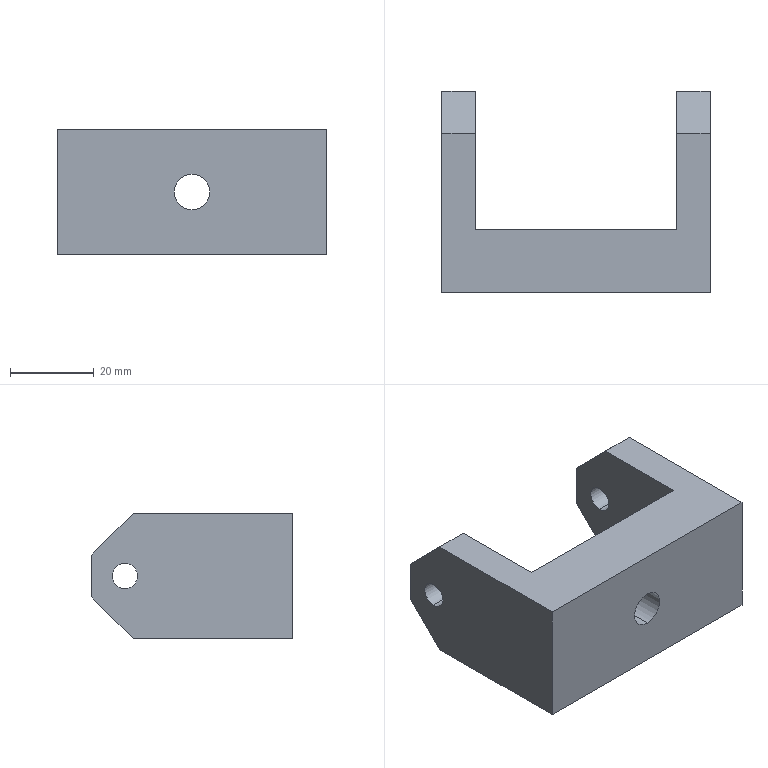Part | STEP file | 0229_205_Joint | 1 solid | 20 faces | box 64 x 48 x 30 mm | volume 41736 mm3 | plane 14 | cylinder 6 | commonest cylinder face diameters 6 x4 8.5 x2
STEP:
#1=CARTESIAN_POINT('',(0.,0.,0.));
#2=DIRECTION('',(0.,0.,1.));
#3=DIRECTION('',(1.,0.,0.));
#4=AXIS2_PLACEMENT_3D('',#1,#2,#3);
#5=CARTESIAN_POINT('',(0.,15.,-19.25));
#6=VERTEX_POINT('',#5);
#7=CARTESIAN_POINT('',(0.,0.,-19.25));
#8=VERTEX_POINT('',#7);
#9=CARTESIAN_POINT('',(0.,0.,-19.25));
#10=DIRECTION('',(0.,-1.,0.));
#11=VECTOR('',#10,1.);
#12=LINE('',#9,#11);
#13=CARTESIAN_POINT('',(0.,0.,-15.));
#14=DIRECTION('',(0.,-1.,0.));
#15=DIRECTION('',(0.,0.,-1.));
#16=AXIS2_PLACEMENT_3D('',#13,#14,#15);
#17=CYLINDRICAL_SURFACE('',#16,4.25);
#18=CARTESIAN_POINT('',(6.283,0.));
#19=DIRECTION('',(0.,1.));
#20=VECTOR('',#19,1.);
#21=LINE('',#18,#20);
#22=(GEOMETRIC_REPRESENTATION_CONTEXT(2)PARAMETRIC_REPRESENTATION_CONTEXT()REPRESENTATION_CONTEXT('',''));
#23=DEFINITIONAL_REPRESENTATION('',(#21),#22);
#24=PCURVE('',#17,#23);
#25=CARTESIAN_POINT('',(0.,0.,-15.));
#26=DIRECTION('',(0.,-1.,0.));
#27=DIRECTION('',(0.,0.,-1.));
#28=AXIS2_PLACEMENT_3D('',#25,#26,#27);
#29=CYLINDRICAL_SURFACE('',#28,4.25);
#30=CARTESIAN_POINT('',(0.,0.));
#31=DIRECTION('',(0.,1.));
#32=VECTOR('',#31,1.);
#33=LINE('',#30,#32);
#34=(GEOMETRIC_REPRESENTATION_CONTEXT(2)PARAMETRIC_REPRESENTATION_CONTEXT()REPRESENTATION_CONTEXT('',''));
#35=DEFINITIONAL_REPRESENTATION('',(#33),#34);
#36=PCURVE('',#29,#35);
#37=SURFACE_CURVE('',#12,(#24,#36),.PCURVE_S1.);
#38=EDGE_CURVE('',#6,#8,#37,.T.);
#39=ORIENTED_EDGE('',*,*,#38,.T.);
#40=CARTESIAN_POINT('',(0.,0.,-10.75));
#41=VERTEX_POINT('',#40);
#42=CARTESIAN_POINT('',(0.,0.,-15.));
#43=DIRECTION('',(0.,-1.,0.));
#44=DIRECTION('',(0.,0.,-1.));
#45=AXIS2_PLACEMENT_3D('',#42,#43,#44);
#46=CIRCLE('',#45,4.25);
#47=CARTESIAN_POINT('',(0.,0.));
#48=DIRECTION('',(1.,0.));
#49=VECTOR('',#48,1.);
#50=LINE('',#47,#49);
#51=(GEOMETRIC_REPRESENTATION_CONTEXT(2)PARAMETRIC_REPRESENTATION_CONTEXT()REPRESENTATION_CONTEXT('',''));
#52=DEFINITIONAL_REPRESENTATION('',(#50),#51);
#53=PCURVE('',#17,#52);
#54=CARTESIAN_POINT('',(-32.,0.,-30.));
#55=DIRECTION('',(0.,-1.,0.));
#56=DIRECTION('',(0.,0.,-1.));
#57=AXIS2_PLACEMENT_3D('',#54,#55,#56);
#58=PLANE('',#57);
#59=CARTESIAN_POINT('',(-15.,32.));
#60=DIRECTION('',(1.,0.));
#61=AXIS2_PLACEMENT_2D('',#59,#60);
#62=CIRCLE('',#61,4.25);
#63=(GEOMETRIC_REPRESENTATION_CONTEXT(2)PARAMETRIC_REPRESENTATION_CONTEXT()REPRESENTATION_CONTEXT('',''));
#64=DEFINITIONAL_REPRESENTATION('',(#62),#63);
#65=PCURVE('',#58,#64);
#66=SURFACE_CURVE('',#46,(#53,#65),.PCURVE_S1.);
#67=EDGE_CURVE('',#41,#8,#66,.T.);
#68=ORIENTED_EDGE('',*,*,#67,.F.);
#69=CARTESIAN_POINT('',(0.,15.,-10.75));
#70=VERTEX_POINT('',#69);
#71=CARTESIAN_POINT('',(0.,0.,-10.75));
#72=DIRECTION('',(0.,-1.,0.));
#73=VECTOR('',#72,1.);
#74=LINE('',#71,#73);
#75=CARTESIAN_POINT('',(3.142,0.));
#76=DIRECTION('',(0.,1.));
#77=VECTOR('',#76,1.);
#78=LINE('',#75,#77);
#79=(GEOMETRIC_REPRESENTATION_CONTEXT(2)PARAMETRIC_REPRESENTATION_CONTEXT()REPRESENTATION_CONTEXT('',''));
#80=DEFINITIONAL_REPRESENTATION('',(#78),#79);
#81=PCURVE('',#17,#80);
#82=CARTESIAN_POINT('',(3.142,0.));
#83=DIRECTION('',(0.,1.));
#84=VECTOR('',#83,1.);
#85=LINE('',#82,#84);
#86=(GEOMETRIC_REPRESENTATION_CONTEXT(2)PARAMETRIC_REPRESENTATION_CONTEXT()REPRESENTATION_CONTEXT('',''));
#87=DEFINITIONAL_REPRESENTATION('',(#85),#86);
#88=PCURVE('',#29,#87);
#89=SURFACE_CURVE('',#74,(#81,#88),.PCURVE_S1.);
#90=EDGE_CURVE('',#70,#41,#89,.T.);
#91=ORIENTED_EDGE('',*,*,#90,.F.);
#92=CARTESIAN_POINT('',(0.,15.,-15.));
#93=DIRECTION('',(0.,-1.,0.));
#94=DIRECTION('',(0.,0.,-1.));
#95=AXIS2_PLACEMENT_3D('',#92,#93,#94);
#96=CIRCLE('',#95,4.25);
#97=CARTESIAN_POINT('',(0.,-15.));
#98=DIRECTION('',(1.,0.));
#99=VECTOR('',#98,1.);
#100=LINE('',#97,#99);
#101=(GEOMETRIC_REPRESENTATION_CONTEXT(2)PARAMETRIC_REPRESENTATION_CONTEXT()REPRESENTATION_CONTEXT('',''));
#102=DEFINITIONAL_REPRESENTATION('',(#100),#101);
#103=PCURVE('',#17,#102);
#104=CARTESIAN_POINT('',(-24.,15.,-30.));
#105=DIRECTION('',(0.,-1.,0.));
#106=DIRECTION('',(0.,0.,-1.));
#107=AXIS2_PLACEMENT_3D('',#104,#105,#106);
#108=PLANE('',#107);
#109=CARTESIAN_POINT('',(-15.,24.));
#110=DIRECTION('',(1.,0.));
#111=AXIS2_PLACEMENT_2D('',#109,#110);
#112=CIRCLE('',#111,4.25);
#113=(GEOMETRIC_REPRESENTATION_CONTEXT(2)PARAMETRIC_REPRESENTATION_CONTEXT()REPRESENTATION_CONTEXT('',''));
#114=DEFINITIONAL_REPRESENTATION('',(#112),#113);
#115=PCURVE('',#108,#114);
#116=SURFACE_CURVE('',#96,(#103,#115),.PCURVE_S1.);
#117=EDGE_CURVE('',#70,#6,#116,.T.);
#118=ORIENTED_EDGE('',*,*,#117,.T.);
#119=EDGE_LOOP('',(#39,#68,#91,#118));
#120=FACE_BOUND('',#119,.F.);
#121=ADVANCED_FACE('',(#120),#17,.F.);
#122=CARTESIAN_POINT('',(-32.,40.,-18.));
#123=VERTEX_POINT('',#122);
#124=CARTESIAN_POINT('',(-24.,40.,-18.));
#125=VERTEX_POINT('',#124);
#126=CARTESIAN_POINT('',(-32.,40.,-18.));
#127=DIRECTION('',(1.,0.,0.));
#128=VECTOR('',#127,1.);
#129=LINE('',#126,#128);
#130=CARTESIAN_POINT('',(-32.,40.,-15.));
#131=DIRECTION('',(1.,0.,0.));
#132=DIRECTION('',(0.,0.,-1.));
#133=AXIS2_PLACEMENT_3D('',#130,#131,#132);
#134=CYLINDRICAL_SURFACE('',#133,3.);
#135=CARTESIAN_POINT('',(6.283,0.));
#136=DIRECTION('',(0.,1.));
#137=VECTOR('',#136,1.);
#138=LINE('',#135,#137);
#139=(GEOMETRIC_REPRESENTATION_CONTEXT(2)PARAMETRIC_REPRESENTATION_CONTEXT()REPRESENTATION_CONTEXT('',''));
#140=DEFINITIONAL_REPRESENTATION('',(#138),#139);
#141=PCURVE('',#134,#140);
#142=CARTESIAN_POINT('',(-32.,40.,-15.));
#143=DIRECTION('',(1.,0.,0.));
#144=DIRECTION('',(0.,0.,-1.));
#145=AXIS2_PLACEMENT_3D('',#142,#143,#144);
#146=CYLINDRICAL_SURFACE('',#145,3.);
#147=CARTESIAN_POINT('',(0.,0.));
#148=DIRECTION('',(0.,1.));
#149=VECTOR('',#148,1.);
#150=LINE('',#147,#149);
#151=(GEOMETRIC_REPRESENTATION_CONTEXT(2)PARAMETRIC_REPRESENTATION_CONTEXT()REPRESENTATION_CONTEXT('',''));
#152=DEFINITIONAL_REPRESENTATION('',(#150),#151);
#153=PCURVE('',#146,#152);
#154=SURFACE_CURVE('',#129,(#141,#153),.PCURVE_S1.);
#155=EDGE_CURVE('',#123,#125,#154,.T.);
#156=ORIENTED_EDGE('',*,*,#155,.T.);
#157=CARTESIAN_POINT('',(-24.,40.,-12.));
#158=VERTEX_POINT('',#157);
#159=CARTESIAN_POINT('',(-24.,40.,-15.));
#160=DIRECTION('',(-1.,0.,0.));
#161=DIRECTION('',(0.,-1.,0.));
#162=AXIS2_PLACEMENT_3D('',#159,#160,#161);
#163=CIRCLE('',#162,3.);
#164=CARTESIAN_POINT('',(10.996,8.));
#165=DIRECTION('',(-1.,0.));
#166=VECTOR('',#165,1.);
#167=LINE('',#164,#166);
#168=(GEOMETRIC_REPRESENTATION_CONTEXT(2)PARAMETRIC_REPRESENTATION_CONTEXT()REPRESENTATION_CONTEXT('',''));
#169=DEFINITIONAL_REPRESENTATION('',(#167),#168);
#170=PCURVE('',#134,#169);
#171=CARTESIAN_POINT('',(-24.,48.,-30.));
#172=DIRECTION('',(-1.,0.,0.));
#173=DIRECTION('',(0.,-1.,0.));
#174=AXIS2_PLACEMENT_3D('',#171,#172,#173);
#175=PLANE('',#174);
#176=CARTESIAN_POINT('',(8.,15.));
#177=DIRECTION('',(1.,0.));
#178=AXIS2_PLACEMENT_2D('',#176,#177);
#179=CIRCLE('',#178,3.);
#180=(GEOMETRIC_REPRESENTATION_CONTEXT(2)PARAMETRIC_REPRESENTATION_CONTEXT()REPRESENTATION_CONTEXT('',''));
#181=DEFINITIONAL_REPRESENTATION('',(#179),#180);
#182=PCURVE('',#175,#181);
#183=SURFACE_CURVE('',#163,(#170,#182),.PCURVE_S1.);
#184=EDGE_CURVE('',#125,#158,#183,.T.);
#185=ORIENTED_EDGE('',*,*,#184,.T.);
#186=CARTESIAN_POINT('',(-32.,40.,-12.));
#187=VERTEX_POINT('',#186);
#188=CARTESIAN_POINT('',(-32.,40.,-12.));
#189=DIRECTION('',(1.,0.,0.));
#190=VECTOR('',#189,1.);
#191=LINE('',#188,#190);
#192=CARTESIAN_POINT('',(3.142,0.));
#193=DIRECTION('',(0.,1.));
#194=VECTOR('',#193,1.);
#195=LINE('',#192,#194);
#196=(GEOMETRIC_REPRESENTATION_CONTEXT(2)PARAMETRIC_REPRESENTATION_CONTEXT()REPRESENTATION_CONTEXT('',''));
#197=DEFINITIONAL_REPRESENTATION('',(#195),#196);
#198=PCURVE('',#134,#197);
#199=CARTESIAN_POINT('',(3.142,0.));
#200=DIRECTION('',(0.,1.));
#201=VECTOR('',#200,1.);
#202=LINE('',#199,#201);
#203=(GEOMETRIC_REPRESENTATION_CONTEXT(2)PARAMETRIC_REPRESENTATION_CONTEXT()REPRESENTATION_CONTEXT('',''));
#204=DEFINITIONAL_REPRESENTATION('',(#202),#203);
#205=PCURVE('',#146,#204);
#206=SURFACE_CURVE('',#191,(#198,#205),.PCURVE_S1.);
#207=EDGE_CURVE('',#187,#158,#206,.T.);
#208=ORIENTED_EDGE('',*,*,#207,.F.);
#209=CARTESIAN_POINT('',(-32.,40.,-15.));
#210=DIRECTION('',(1.,0.,0.));
#211=DIRECTION('',(0.,0.,-1.));
#212=AXIS2_PLACEMENT_3D('',#209,#210,#211);
#213=CIRCLE('',#212,3.);
#214=CARTESIAN_POINT('',(0.,0.));
#215=DIRECTION('',(1.,0.));
#216=VECTOR('',#215,1.);
#217=LINE('',#214,#216);
#218=(GEOMETRIC_REPRESENTATION_CONTEXT(2)PARAMETRIC_REPRESENTATION_CONTEXT()REPRESENTATION_CONTEXT('',''));
#219=DEFINITIONAL_REPRESENTATION('',(#217),#218);
#220=PCURVE('',#134,#219);
#221=CARTESIAN_POINT('',(-32.,48.,-30.));
#222=DIRECTION('',(-1.,0.,0.));
#223=DIRECTION('',(0.,0.,1.));
#224=AXIS2_PLACEMENT_3D('',#221,#222,#223);
#225=PLANE('',#224);
#226=CARTESIAN_POINT('',(12.,-8.));
#227=CARTESIAN_POINT('',(12.,-2.804));
#228=CARTESIAN_POINT('',(16.5,-5.402));
#229=CARTESIAN_POINT('',(21.,-8.));
#230=CARTESIAN_POINT('',(16.5,-10.598));
#231=CARTESIAN_POINT('',(12.,-13.196));
#232=CARTESIAN_POINT('',(12.,-8.));
#233=(BOUNDED_CURVE()B_SPLINE_CURVE(2,(#226,#227,#228,#229,#230,#231,#232),.UNSPECIFIED.,.T.,.F.)B_SPLINE_CURVE_WITH_KNOTS((1,2,2,2,2,1),(-2.094,0.,2.094,4.189,6.283,8.378),.UNSPECIFIED.)CURVE()GEOMETRIC_REPRESENTATION_ITEM()RATIONAL_B_SPLINE_CURVE((1.,0.5,1.,0.5,1.,0.5,1.))REPRESENTATION_ITEM(''));
#234=(GEOMETRIC_REPRESENTATION_CONTEXT(2)PARAMETRIC_REPRESENTATION_CONTEXT()REPRESENTATION_CONTEXT('',''));
#235=DEFINITIONAL_REPRESENTATION('',(#233),#234);
#236=PCURVE('',#225,#235);
#237=SURFACE_CURVE('',#213,(#220,#236),.PCURVE_S1.);
#238=EDGE_CURVE('',#187,#123,#237,.T.);
#239=ORIENTED_EDGE('',*,*,#238,.T.);
#240=EDGE_LOOP('',(#156,#185,#208,#239));
#241=FACE_BOUND('',#240,.F.);
#242=ADVANCED_FACE('',(#241),#134,.F.);
#243=CARTESIAN_POINT('',(24.,40.,-18.));
#244=VERTEX_POINT('',#243);
#245=CARTESIAN_POINT('',(32.,40.,-18.));
#246=VERTEX_POINT('',#245);
#247=CARTESIAN_POINT('',(-32.,40.,-18.));
#248=DIRECTION('',(1.,0.,0.));
#249=VECTOR('',#248,1.);
#250=LINE('',#247,#249);
#251=CARTESIAN_POINT('',(-32.,40.,-15.));
#252=DIRECTION('',(1.,0.,0.));
#253=DIRECTION('',(0.,0.,-1.));
#254=AXIS2_PLACEMENT_3D('',#251,#252,#253);
#255=CYLINDRICAL_SURFACE('',#254,3.);
#256=CARTESIAN_POINT('',(6.283,0.));
#257=DIRECTION('',(0.,1.));
#258=VECTOR('',#257,1.);
#259=LINE('',#256,#258);
#260=(GEOMETRIC_REPRESENTATION_CONTEXT(2)PARAMETRIC_REPRESENTATION_CONTEXT()REPRESENTATION_CONTEXT('',''));
#261=DEFINITIONAL_REPRESENTATION('',(#259),#260);
#262=PCURVE('',#255,#261);
#263=CARTESIAN_POINT('',(-32.,40.,-15.));
#264=DIRECTION('',(1.,0.,0.));
#265=DIRECTION('',(0.,0.,-1.));
#266=AXIS2_PLACEMENT_3D('',#263,#264,#265);
#267=CYLINDRICAL_SURFACE('',#266,3.);
#268=CARTESIAN_POINT('',(0.,0.));
#269=DIRECTION('',(0.,1.));
#270=VECTOR('',#269,1.);
#271=LINE('',#268,#270);
#272=(GEOMETRIC_REPRESENTATION_CONTEXT(2)PARAMETRIC_REPRESENTATION_CONTEXT()REPRESENTATION_CONTEXT('',''));
#273=DEFINITIONAL_REPRESENTATION('',(#271),#272);
#274=PCURVE('',#267,#273);
#275=SURFACE_CURVE('',#250,(#262,#274),.PCURVE_S1.);
#276=EDGE_CURVE('',#244,#246,#275,.T.);
#277=ORIENTED_EDGE('',*,*,#276,.T.);
#278=CARTESIAN_POINT('',(32.,40.,-12.));
#279=VERTEX_POINT('',#278);
#280=CARTESIAN_POINT('',(32.,40.,-15.));
#281=DIRECTION('',(1.,0.,0.));
#282=DIRECTION('',(0.,0.,-1.));
#283=AXIS2_PLACEMENT_3D('',#280,#281,#282);
#284=CIRCLE('',#283,3.);
#285=CARTESIAN_POINT('',(0.,64.));
#286=DIRECTION('',(1.,0.));
#287=VECTOR('',#286,1.);
#288=LINE('',#285,#287);
#289=(GEOMETRIC_REPRESENTATION_CONTEXT(2)PARAMETRIC_REPRESENTATION_CONTEXT()REPRESENTATION_CONTEXT('',''));
#290=DEFINITIONAL_REPRESENTATION('',(#288),#289);
#291=PCURVE('',#255,#290);
#292=CARTESIAN_POINT('',(32.,48.,-30.));
#293=DIRECTION('',(1.,0.,0.));
#294=DIRECTION('',(0.,0.,-1.));
#295=AXIS2_PLACEMENT_3D('',#292,#293,#294);
#296=PLANE('',#295);
#297=CARTESIAN_POINT('',(-15.,-8.));
#298=DIRECTION('',(1.,0.));
#299=AXIS2_PLACEMENT_2D('',#297,#298);
#300=CIRCLE('',#299,3.);
#301=(GEOMETRIC_REPRESENTATION_CONTEXT(2)PARAMETRIC_REPRESENTATION_CONTEXT()REPRESENTATION_CONTEXT('',''));
#302=DEFINITIONAL_REPRESENTATION('',(#300),#301);
#303=PCURVE('',#296,#302);
#304=SURFACE_CURVE('',#284,(#291,#303),.PCURVE_S1.);
#305=EDGE_CURVE('',#279,#246,#304,.T.);
#306=ORIENTED_EDGE('',*,*,#305,.F.);
#307=CARTESIAN_POINT('',(24.,40.,-12.));
#308=VERTEX_POINT('',#307);
#309=CARTESIAN_POINT('',(-32.,40.,-12.));
#310=DIRECTION('',(1.,0.,0.));
#311=VECTOR('',#310,1.);
#312=LINE('',#309,#311);
#313=CARTESIAN_POINT('',(3.142,0.));
#314=DIRECTION('',(0.,1.));
#315=VECTOR('',#314,1.);
#316=LINE('',#313,#315);
#317=(GEOMETRIC_REPRESENTATION_CONTEXT(2)PARAMETRIC_REPRESENTATION_CONTEXT()REPRESENTATION_CONTEXT('',''));
#318=DEFINITIONAL_REPRESENTATION('',(#316),#317);
#319=PCURVE('',#255,#318);
#320=CARTESIAN_POINT('',(3.142,0.));
#321=DIRECTION('',(0.,1.));
#322=VECTOR('',#321,1.);
#323=LINE('',#320,#322);
#324=(GEOMETRIC_REPRESENTATION_CONTEXT(2)PARAMETRIC_REPRESENTATION_CONTEXT()REPRESENTATION_CONTEXT('',''));
#325=DEFINITIONAL_REPRESENTATION('',(#323),#324);
#326=PCURVE('',#267,#325);
#327=SURFACE_CURVE('',#312,(#319,#326),.PCURVE_S1.);
#328=EDGE_CURVE('',#308,#279,#327,.T.);
#329=ORIENTED_EDGE('',*,*,#328,.F.);
#330=CARTESIAN_POINT('',(24.,40.,-15.));
#331=DIRECTION('',(1.,0.,0.));
#332=DIRECTION('',(0.,1.,0.));
#333=AXIS2_PLACEMENT_3D('',#330,#331,#332);
#334=CIRCLE('',#333,3.);
#335=CARTESIAN_POINT('',(1.571,56.));
#336=DIRECTION('',(1.,0.));
#337=VECTOR('',#336,1.);
#338=LINE('',#335,#337);
#339=(GEOMETRIC_REPRESENTATION_CONTEXT(2)PARAMETRIC_REPRESENTATION_CONTEXT()REPRESENTATION_CONTEXT('',''));
#340=DEFINITIONAL_REPRESENTATION('',(#338),#339);
#341=PCURVE('',#255,#340);
#342=CARTESIAN_POINT('',(24.,48.,-30.));
#343=DIRECTION('',(1.,0.,0.));
#344=DIRECTION('',(0.,1.,0.));
#345=AXIS2_PLACEMENT_3D('',#342,#343,#344);
#346=PLANE('',#345);
#347=CARTESIAN_POINT('',(-8.,15.));
#348=DIRECTION('',(1.,0.));
#349=AXIS2_PLACEMENT_2D('',#347,#348);
#350=CIRCLE('',#349,3.);
#351=(GEOMETRIC_REPRESENTATION_CONTEXT(2)PARAMETRIC_REPRESENTATION_CONTEXT()REPRESENTATION_CONTEXT('',''));
#352=DEFINITIONAL_REPRESENTATION('',(#350),#351);
#353=PCURVE('',#346,#352);
#354=SURFACE_CURVE('',#334,(#341,#353),.PCURVE_S1.);
#355=EDGE_CURVE('',#308,#244,#354,.T.);
#356=ORIENTED_EDGE('',*,*,#355,.T.);
#357=EDGE_LOOP('',(#277,#306,#329,#356));
#358=FACE_BOUND('',#357,.F.);
#359=ADVANCED_FACE('',(#358),#255,.F.);
#360=CARTESIAN_POINT('',(-24.,48.,-20.));
#361=VERTEX_POINT('',#360);
#362=CARTESIAN_POINT('',(-24.,48.,-10.));
#363=VERTEX_POINT('',#362);
#364=CARTESIAN_POINT('',(-24.,48.,-30.));
#365=DIRECTION('',(0.,0.,1.));
#366=VECTOR('',#365,1.);
#367=LINE('',#364,#366);
#368=CARTESIAN_POINT('',(-32.,48.,-30.));
#369=DIRECTION('',(0.,1.,0.));
#370=DIRECTION('',(0.,0.,1.));
#371=AXIS2_PLACEMENT_3D('',#368,#369,#370);
#372=PLANE('',#371);
#373=CARTESIAN_POINT('',(0.,8.));
#374=DIRECTION('',(1.,0.));
#375=VECTOR('',#374,1.);
#376=LINE('',#373,#375);
#377=(GEOMETRIC_REPRESENTATION_CONTEXT(2)PARAMETRIC_REPRESENTATION_CONTEXT()REPRESENTATION_CONTEXT('',''));
#378=DEFINITIONAL_REPRESENTATION('',(#376),#377);
#379=PCURVE('',#372,#378);
#380=CARTESIAN_POINT('',(0.,0.));
#381=DIRECTION('',(0.,1.));
#382=VECTOR('',#381,1.);
#383=LINE('',#380,#382);
#384=(GEOMETRIC_REPRESENTATION_CONTEXT(2)PARAMETRIC_REPRESENTATION_CONTEXT()REPRESENTATION_CONTEXT('',''));
#385=DEFINITIONAL_REPRESENTATION('',(#383),#384);
#386=PCURVE('',#175,#385);
#387=SURFACE_CURVE('',#367,(#379,#386),.PCURVE_S1.);
#388=EDGE_CURVE('',#361,#363,#387,.T.);
#389=ORIENTED_EDGE('',*,*,#388,.F.);
#390=CARTESIAN_POINT('',(-32.,48.,-20.));
#391=VERTEX_POINT('',#390);
#392=CARTESIAN_POINT('',(-32.,48.,-20.));
#393=DIRECTION('',(-1.,0.,0.));
#394=VECTOR('',#393,1.);
#395=LINE('',#392,#394);
#396=CARTESIAN_POINT('',(10.,0.));
#397=DIRECTION('',(0.,-1.));
#398=VECTOR('',#397,1.);
#399=LINE('',#396,#398);
#400=(GEOMETRIC_REPRESENTATION_CONTEXT(2)PARAMETRIC_REPRESENTATION_CONTEXT()REPRESENTATION_CONTEXT('',''));
#401=DEFINITIONAL_REPRESENTATION('',(#399),#400);
#402=PCURVE('',#372,#401);
#403=CARTESIAN_POINT('',(-32.,48.,-20.));
#404=DIRECTION('',(0.,0.7071,-0.7071));
#405=DIRECTION('',(0.,0.7071,0.7071));
#406=AXIS2_PLACEMENT_3D('',#403,#404,#405);
#407=PLANE('',#406);
#408=CARTESIAN_POINT('',(0.,0.));
#409=DIRECTION('',(0.,-1.));
#410=VECTOR('',#409,1.);
#411=LINE('',#408,#410);
#412=(GEOMETRIC_REPRESENTATION_CONTEXT(2)PARAMETRIC_REPRESENTATION_CONTEXT()REPRESENTATION_CONTEXT('',''));
#413=DEFINITIONAL_REPRESENTATION('',(#411),#412);
#414=PCURVE('',#407,#413);
#415=SURFACE_CURVE('',#395,(#402,#414),.PCURVE_S1.);
#416=EDGE_CURVE('',#361,#391,#415,.T.);
#417=ORIENTED_EDGE('',*,*,#416,.T.);
#418=CARTESIAN_POINT('',(-32.,48.,-10.));
#419=VERTEX_POINT('',#418);
#420=CARTESIAN_POINT('',(-32.,48.,-30.));
#421=DIRECTION('',(0.,0.,1.));
#422=VECTOR('',#421,1.);
#423=LINE('',#420,#422);
#424=CARTESIAN_POINT('',(0.,0.));
#425=DIRECTION('',(1.,0.));
#426=VECTOR('',#425,1.);
#427=LINE('',#424,#426);
#428=(GEOMETRIC_REPRESENTATION_CONTEXT(2)PARAMETRIC_REPRESENTATION_CONTEXT()REPRESENTATION_CONTEXT('',''));
#429=DEFINITIONAL_REPRESENTATION('',(#427),#428);
#430=PCURVE('',#372,#429);
#431=CARTESIAN_POINT('',(0.,0.));
#432=DIRECTION('',(1.,0.));
#433=VECTOR('',#432,1.);
#434=LINE('',#431,#433);
#435=(GEOMETRIC_REPRESENTATION_CONTEXT(2)PARAMETRIC_REPRESENTATION_CONTEXT()REPRESENTATION_CONTEXT('',''));
#436=DEFINITIONAL_REPRESENTATION('',(#434),#435);
#437=PCURVE('',#225,#436);
#438=SURFACE_CURVE('',#423,(#430,#437),.PCURVE_S1.);
#439=EDGE_CURVE('',#391,#419,#438,.T.);
#440=ORIENTED_EDGE('',*,*,#439,.T.);
#441=CARTESIAN_POINT('',(-32.,48.,-10.));
#442=DIRECTION('',(1.,0.,0.));
#443=VECTOR('',#442,1.);
#444=LINE('',#441,#443);
#445=CARTESIAN_POINT('',(20.,0.));
#446=DIRECTION('',(0.,1.));
#447=VECTOR('',#446,1.);
#448=LINE('',#445,#447);
#449=(GEOMETRIC_REPRESENTATION_CONTEXT(2)PARAMETRIC_REPRESENTATION_CONTEXT()REPRESENTATION_CONTEXT('',''));
#450=DEFINITIONAL_REPRESENTATION('',(#448),#449);
#451=PCURVE('',#372,#450);
#452=CARTESIAN_POINT('',(-32.,38.,0.));
#453=DIRECTION('',(0.,-0.7071,-0.7071));
#454=DIRECTION('',(0.,0.7071,-0.7071));
#455=AXIS2_PLACEMENT_3D('',#452,#453,#454);
#456=PLANE('',#455);
#457=CARTESIAN_POINT('',(14.142,0.));
#458=DIRECTION('',(0.,1.));
#459=VECTOR('',#458,1.);
#460=LINE('',#457,#459);
#461=(GEOMETRIC_REPRESENTATION_CONTEXT(2)PARAMETRIC_REPRESENTATION_CONTEXT()REPRESENTATION_CONTEXT('',''));
#462=DEFINITIONAL_REPRESENTATION('',(#460),#461);
#463=PCURVE('',#456,#462);
#464=SURFACE_CURVE('',#444,(#451,#463),.PCURVE_S1.);
#465=EDGE_CURVE('',#419,#363,#464,.T.);
#466=ORIENTED_EDGE('',*,*,#465,.T.);
#467=EDGE_LOOP('',(#389,#417,#440,#466));
#468=FACE_BOUND('',#467,.T.);
#469=ADVANCED_FACE('',(#468),#372,.T.);
#470=CARTESIAN_POINT('',(-32.,40.,-15.));
#471=DIRECTION('',(1.,0.,0.));
#472=DIRECTION('',(0.,0.,-1.));
#473=AXIS2_PLACEMENT_3D('',#470,#471,#472);
#474=CIRCLE('',#473,3.);
#475=CARTESIAN_POINT('',(12.,-8.));
#476=CARTESIAN_POINT('',(12.,-2.804));
#477=CARTESIAN_POINT('',(16.5,-5.402));
#478=CARTESIAN_POINT('',(21.,-8.));
#479=CARTESIAN_POINT('',(16.5,-10.598));
#480=CARTESIAN_POINT('',(12.,-13.196));
#481=CARTESIAN_POINT('',(12.,-8.));
#482=(BOUNDED_CURVE()B_SPLINE_CURVE(2,(#475,#476,#477,#478,#479,#480,#481),.UNSPECIFIED.,.T.,.F.)B_SPLINE_CURVE_WITH_KNOTS((1,2,2,2,2,1),(-2.094,0.,2.094,4.189,6.283,8.378),.UNSPECIFIED.)CURVE()GEOMETRIC_REPRESENTATION_ITEM()RATIONAL_B_SPLINE_CURVE((1.,0.5,1.,0.5,1.,0.5,1.))REPRESENTATION_ITEM(''));
#483=(GEOMETRIC_REPRESENTATION_CONTEXT(2)PARAMETRIC_REPRESENTATION_CONTEXT()REPRESENTATION_CONTEXT('',''));
#484=DEFINITIONAL_REPRESENTATION('',(#482),#483);
#485=PCURVE('',#225,#484);
#486=CARTESIAN_POINT('',(0.,0.));
#487=DIRECTION('',(1.,0.));
#488=VECTOR('',#487,1.);
#489=LINE('',#486,#488);
#490=(GEOMETRIC_REPRESENTATION_CONTEXT(2)PARAMETRIC_REPRESENTATION_CONTEXT()REPRESENTATION_CONTEXT('',''));
#491=DEFINITIONAL_REPRESENTATION('',(#489),#490);
#492=PCURVE('',#146,#491);
#493=SURFACE_CURVE('',#474,(#485,#492),.PCURVE_S1.);
#494=EDGE_CURVE('',#123,#187,#493,.T.);
#495=ORIENTED_EDGE('',*,*,#494,.T.);
#496=ORIENTED_EDGE('',*,*,#238,.T.);
#497=EDGE_LOOP('',(#495,#496));
#498=FACE_BOUND('',#497,.T.);
#499=ORIENTED_EDGE('',*,*,#439,.F.);
#500=CARTESIAN_POINT('',(-32.,38.,-30.));
#501=VERTEX_POINT('',#500);
#502=CARTESIAN_POINT('',(-32.,43.,-25.));
#503=DIRECTION('',(0.,-0.7071,-0.7071));
#504=VECTOR('',#503,1.);
#505=LINE('',#502,#504);
#506=CARTESIAN_POINT('',(5.,-5.));
#507=DIRECTION('',(-0.7071,-0.7071));
#508=VECTOR('',#507,1.);
#509=LINE('',#506,#508);
#510=(GEOMETRIC_REPRESENTATION_CONTEXT(2)PARAMETRIC_REPRESENTATION_CONTEXT()REPRESENTATION_CONTEXT('',''));
#511=DEFINITIONAL_REPRESENTATION('',(#509),#510);
#512=PCURVE('',#225,#511);
#513=CARTESIAN_POINT('',(-7.071,0.));
#514=DIRECTION('',(-1.,0.));
#515=VECTOR('',#514,1.);
#516=LINE('',#513,#515);
#517=(GEOMETRIC_REPRESENTATION_CONTEXT(2)PARAMETRIC_REPRESENTATION_CONTEXT()REPRESENTATION_CONTEXT('',''));
#518=DEFINITIONAL_REPRESENTATION('',(#516),#517);
#519=PCURVE('',#407,#518);
#520=SURFACE_CURVE('',#505,(#512,#519),.PCURVE_S1.);
#521=EDGE_CURVE('',#391,#501,#520,.T.);
#522=ORIENTED_EDGE('',*,*,#521,.T.);
#523=CARTESIAN_POINT('',(-32.,0.,-30.));
#524=VERTEX_POINT('',#523);
#525=CARTESIAN_POINT('',(-32.,48.,-30.));
#526=DIRECTION('',(0.,-1.,0.));
#527=VECTOR('',#526,1.);
#528=LINE('',#525,#527);
#529=CARTESIAN_POINT('',(0.,0.));
#530=DIRECTION('',(0.,-1.));
#531=VECTOR('',#530,1.);
#532=LINE('',#529,#531);
#533=(GEOMETRIC_REPRESENTATION_CONTEXT(2)PARAMETRIC_REPRESENTATION_CONTEXT()REPRESENTATION_CONTEXT('',''));
#534=DEFINITIONAL_REPRESENTATION('',(#532),#533);
#535=PCURVE('',#225,#534);
#536=CARTESIAN_POINT('',(-32.,0.,-30.));
#537=DIRECTION('',(0.,0.,1.));
#538=DIRECTION('',(1.,0.,0.));
#539=AXIS2_PLACEMENT_3D('',#536,#537,#538);
#540=PLANE('',#539);
#541=CARTESIAN_POINT('',(0.,48.));
#542=DIRECTION('',(0.,-1.));
#543=VECTOR('',#542,1.);
#544=LINE('',#541,#543);
#545=(GEOMETRIC_REPRESENTATION_CONTEXT(2)PARAMETRIC_REPRESENTATION_CONTEXT()REPRESENTATION_CONTEXT('',''));
#546=DEFINITIONAL_REPRESENTATION('',(#544),#545);
#547=PCURVE('',#540,#546);
#548=SURFACE_CURVE('',#528,(#535,#547),.PCURVE_S1.);
#549=EDGE_CURVE('',#501,#524,#548,.T.);
#550=ORIENTED_EDGE('',*,*,#549,.T.);
#551=CARTESIAN_POINT('',(-32.,0.,0.));
#552=VERTEX_POINT('',#551);
#553=CARTESIAN_POINT('',(-32.,0.,-30.));
#554=DIRECTION('',(0.,0.,1.));
#555=VECTOR('',#554,1.);
#556=LINE('',#553,#555);
#557=CARTESIAN_POINT('',(0.,-48.));
#558=DIRECTION('',(1.,0.));
#559=VECTOR('',#558,1.);
#560=LINE('',#557,#559);
#561=(GEOMETRIC_REPRESENTATION_CONTEXT(2)PARAMETRIC_REPRESENTATION_CONTEXT()REPRESENTATION_CONTEXT('',''));
#562=DEFINITIONAL_REPRESENTATION('',(#560),#561);
#563=PCURVE('',#225,#562);
#564=CARTESIAN_POINT('',(0.,0.));
#565=DIRECTION('',(-1.,0.));
#566=VECTOR('',#565,1.);
#567=LINE('',#564,#566);
#568=(GEOMETRIC_REPRESENTATION_CONTEXT(2)PARAMETRIC_REPRESENTATION_CONTEXT()REPRESENTATION_CONTEXT('',''));
#569=DEFINITIONAL_REPRESENTATION('',(#567),#568);
#570=PCURVE('',#58,#569);
#571=SURFACE_CURVE('',#556,(#563,#570),.PCURVE_S1.);
#572=EDGE_CURVE('',#524,#552,#571,.T.);
#573=ORIENTED_EDGE('',*,*,#572,.T.);
#574=CARTESIAN_POINT('',(-32.,38.,0.));
#575=VERTEX_POINT('',#574);
#576=CARTESIAN_POINT('',(-32.,48.,0.));
#577=DIRECTION('',(0.,-1.,0.));
#578=VECTOR('',#577,1.);
#579=LINE('',#576,#578);
#580=CARTESIAN_POINT('',(30.,0.));
#581=DIRECTION('',(0.,-1.));
#582=VECTOR('',#581,1.);
#583=LINE('',#580,#582);
#584=(GEOMETRIC_REPRESENTATION_CONTEXT(2)PARAMETRIC_REPRESENTATION_CONTEXT()REPRESENTATION_CONTEXT('',''));
#585=DEFINITIONAL_REPRESENTATION('',(#583),#584);
#586=PCURVE('',#225,#585);
#587=CARTESIAN_POINT('',(-32.,0.,0.));
#588=DIRECTION('',(0.,0.,1.));
#589=DIRECTION('',(1.,0.,0.));
#590=AXIS2_PLACEMENT_3D('',#587,#588,#589);
#591=PLANE('',#590);
#592=CARTESIAN_POINT('',(0.,48.));
#593=DIRECTION('',(0.,-1.));
#594=VECTOR('',#593,1.);
#595=LINE('',#592,#594);
#596=(GEOMETRIC_REPRESENTATION_CONTEXT(2)PARAMETRIC_REPRESENTATION_CONTEXT()REPRESENTATION_CONTEXT('',''));
#597=DEFINITIONAL_REPRESENTATION('',(#595),#596);
#598=PCURVE('',#591,#597);
#599=SURFACE_CURVE('',#579,(#586,#598),.PCURVE_S1.);
#600=EDGE_CURVE('',#575,#552,#599,.T.);
#601=ORIENTED_EDGE('',*,*,#600,.F.);
#602=CARTESIAN_POINT('',(-32.,58.,-20.));
#603=DIRECTION('',(0.,0.7071,-0.7071));
#604=VECTOR('',#603,1.);
#605=LINE('',#602,#604);
#606=CARTESIAN_POINT('',(10.,10.));
#607=DIRECTION('',(-0.7071,0.7071));
#608=VECTOR('',#607,1.);
#609=LINE('',#606,#608);
#610=(GEOMETRIC_REPRESENTATION_CONTEXT(2)PARAMETRIC_REPRESENTATION_CONTEXT()REPRESENTATION_CONTEXT('',''));
#611=DEFINITIONAL_REPRESENTATION('',(#609),#610);
#612=PCURVE('',#225,#611);
#613=CARTESIAN_POINT('',(28.284,0.));
#614=DIRECTION('',(1.,0.));
#615=VECTOR('',#614,1.);
#616=LINE('',#613,#615);
#617=(GEOMETRIC_REPRESENTATION_CONTEXT(2)PARAMETRIC_REPRESENTATION_CONTEXT()REPRESENTATION_CONTEXT('',''));
#618=DEFINITIONAL_REPRESENTATION('',(#616),#617);
#619=PCURVE('',#456,#618);
#620=SURFACE_CURVE('',#605,(#612,#619),.PCURVE_S1.);
#621=EDGE_CURVE('',#575,#419,#620,.T.);
#622=ORIENTED_EDGE('',*,*,#621,.T.);
#623=EDGE_LOOP('',(#499,#522,#550,#573,#601,#622));
#624=FACE_BOUND('',#623,.T.);
#625=ADVANCED_FACE('',(#498,#624),#225,.T.);
#626=CARTESIAN_POINT('',(32.,48.,-20.));
#627=VERTEX_POINT('',#626);
#628=CARTESIAN_POINT('',(32.,48.,-10.));
#629=VERTEX_POINT('',#628);
#630=CARTESIAN_POINT('',(32.,48.,-30.));
#631=DIRECTION('',(0.,0.,1.));
#632=VECTOR('',#631,1.);
#633=LINE('',#630,#632);
#634=CARTESIAN_POINT('',(-32.,48.,-30.));
#635=DIRECTION('',(0.,1.,0.));
#636=DIRECTION('',(0.,0.,1.));
#637=AXIS2_PLACEMENT_3D('',#634,#635,#636);
#638=PLANE('',#637);
#639=CARTESIAN_POINT('',(0.,64.));
#640=DIRECTION('',(1.,0.));
#641=VECTOR('',#640,1.);
#642=LINE('',#639,#641);
#643=(GEOMETRIC_REPRESENTATION_CONTEXT(2)PARAMETRIC_REPRESENTATION_CONTEXT()REPRESENTATION_CONTEXT('',''));
#644=DEFINITIONAL_REPRESENTATION('',(#642),#643);
#645=PCURVE('',#638,#644);
#646=CARTESIAN_POINT('',(0.,0.));
#647=DIRECTION('',(-1.,0.));
#648=VECTOR('',#647,1.);
#649=LINE('',#646,#648);
#650=(GEOMETRIC_REPRESENTATION_CONTEXT(2)PARAMETRIC_REPRESENTATION_CONTEXT()REPRESENTATION_CONTEXT('',''));
#651=DEFINITIONAL_REPRESENTATION('',(#649),#650);
#652=PCURVE('',#296,#651);
#653=SURFACE_CURVE('',#633,(#645,#652),.PCURVE_S1.);
#654=EDGE_CURVE('',#627,#629,#653,.T.);
#655=ORIENTED_EDGE('',*,*,#654,.F.);
#656=CARTESIAN_POINT('',(24.,48.,-20.));
#657=VERTEX_POINT('',#656);
#658=CARTESIAN_POINT('',(24.,48.,-20.));
#659=DIRECTION('',(-1.,0.,0.));
#660=VECTOR('',#659,1.);
#661=LINE('',#658,#660);
#662=CARTESIAN_POINT('',(10.,56.));
#663=DIRECTION('',(0.,-1.));
#664=VECTOR('',#663,1.);
#665=LINE('',#662,#664);
#666=(GEOMETRIC_REPRESENTATION_CONTEXT(2)PARAMETRIC_REPRESENTATION_CONTEXT()REPRESENTATION_CONTEXT('',''));
#667=DEFINITIONAL_REPRESENTATION('',(#665),#666);
#668=PCURVE('',#638,#667);
#669=CARTESIAN_POINT('',(-32.,48.,-20.));
#670=DIRECTION('',(0.,0.7071,-0.7071));
#671=DIRECTION('',(0.,0.7071,0.7071));
#672=AXIS2_PLACEMENT_3D('',#669,#670,#671);
#673=PLANE('',#672);
#674=CARTESIAN_POINT('',(0.,56.));
#675=DIRECTION('',(0.,-1.));
#676=VECTOR('',#675,1.);
#677=LINE('',#674,#676);
#678=(GEOMETRIC_REPRESENTATION_CONTEXT(2)PARAMETRIC_REPRESENTATION_CONTEXT()REPRESENTATION_CONTEXT('',''));
#679=DEFINITIONAL_REPRESENTATION('',(#677),#678);
#680=PCURVE('',#673,#679);
#681=SURFACE_CURVE('',#661,(#668,#680),.PCURVE_S1.);
#682=EDGE_CURVE('',#627,#657,#681,.T.);
#683=ORIENTED_EDGE('',*,*,#682,.T.);
#684=CARTESIAN_POINT('',(24.,48.,-10.));
#685=VERTEX_POINT('',#684);
#686=CARTESIAN_POINT('',(24.,48.,-30.));
#687=DIRECTION('',(0.,0.,1.));
#688=VECTOR('',#687,1.);
#689=LINE('',#686,#688);
#690=CARTESIAN_POINT('',(0.,56.));
#691=DIRECTION('',(1.,0.));
#692=VECTOR('',#691,1.);
#693=LINE('',#690,#692);
#694=(GEOMETRIC_REPRESENTATION_CONTEXT(2)PARAMETRIC_REPRESENTATION_CONTEXT()REPRESENTATION_CONTEXT('',''));
#695=DEFINITIONAL_REPRESENTATION('',(#693),#694);
#696=PCURVE('',#638,#695);
#697=CARTESIAN_POINT('',(0.,0.));
#698=DIRECTION('',(0.,1.));
#699=VECTOR('',#698,1.);
#700=LINE('',#697,#699);
#701=(GEOMETRIC_REPRESENTATION_CONTEXT(2)PARAMETRIC_REPRESENTATION_CONTEXT()REPRESENTATION_CONTEXT('',''));
#702=DEFINITIONAL_REPRESENTATION('',(#700),#701);
#703=PCURVE('',#346,#702);
#704=SURFACE_CURVE('',#689,(#696,#703),.PCURVE_S1.);
#705=EDGE_CURVE('',#657,#685,#704,.T.);
#706=ORIENTED_EDGE('',*,*,#705,.T.);
#707=CARTESIAN_POINT('',(-32.,48.,-10.));
#708=DIRECTION('',(1.,0.,0.));
#709=VECTOR('',#708,1.);
#710=LINE('',#707,#709);
#711=CARTESIAN_POINT('',(20.,0.));
#712=DIRECTION('',(0.,1.));
#713=VECTOR('',#712,1.);
#714=LINE('',#711,#713);
#715=(GEOMETRIC_REPRESENTATION_CONTEXT(2)PARAMETRIC_REPRESENTATION_CONTEXT()REPRESENTATION_CONTEXT('',''));
#716=DEFINITIONAL_REPRESENTATION('',(#714),#715);
#717=PCURVE('',#638,#716);
#718=CARTESIAN_POINT('',(-32.,38.,0.));
#719=DIRECTION('',(0.,-0.7071,-0.7071));
#720=DIRECTION('',(0.,0.7071,-0.7071));
#721=AXIS2_PLACEMENT_3D('',#718,#719,#720);
#722=PLANE('',#721);
#723=CARTESIAN_POINT('',(14.142,0.));
#724=DIRECTION('',(0.,1.));
#725=VECTOR('',#724,1.);
#726=LINE('',#723,#725);
#727=(GEOMETRIC_REPRESENTATION_CONTEXT(2)PARAMETRIC_REPRESENTATION_CONTEXT()REPRESENTATION_CONTEXT('',''));
#728=DEFINITIONAL_REPRESENTATION('',(#726),#727);
#729=PCURVE('',#722,#728);
#730=SURFACE_CURVE('',#710,(#717,#729),.PCURVE_S1.);
#731=EDGE_CURVE('',#685,#629,#730,.T.);
#732=ORIENTED_EDGE('',*,*,#731,.T.);
#733=EDGE_LOOP('',(#655,#683,#706,#732));
#734=FACE_BOUND('',#733,.T.);
#735=ADVANCED_FACE('',(#734),#638,.T.);
#736=CARTESIAN_POINT('',(32.,40.,-15.));
#737=DIRECTION('',(1.,0.,0.));
#738=DIRECTION('',(0.,0.,-1.));
#739=AXIS2_PLACEMENT_3D('',#736,#737,#738);
#740=CIRCLE('',#739,3.);
#741=CARTESIAN_POINT('',(-15.,-8.));
#742=DIRECTION('',(1.,0.));
#743=AXIS2_PLACEMENT_2D('',#741,#742);
#744=CIRCLE('',#743,3.);
#745=(GEOMETRIC_REPRESENTATION_CONTEXT(2)PARAMETRIC_REPRESENTATION_CONTEXT()REPRESENTATION_CONTEXT('',''));
#746=DEFINITIONAL_REPRESENTATION('',(#744),#745);
#747=PCURVE('',#296,#746);
#748=CARTESIAN_POINT('',(0.,64.));
#749=DIRECTION('',(1.,0.));
#750=VECTOR('',#749,1.);
#751=LINE('',#748,#750);
#752=(GEOMETRIC_REPRESENTATION_CONTEXT(2)PARAMETRIC_REPRESENTATION_CONTEXT()REPRESENTATION_CONTEXT('',''));
#753=DEFINITIONAL_REPRESENTATION('',(#751),#752);
#754=PCURVE('',#267,#753);
#755=SURFACE_CURVE('',#740,(#747,#754),.PCURVE_S1.);
#756=EDGE_CURVE('',#246,#279,#755,.T.);
#757=ORIENTED_EDGE('',*,*,#756,.F.);
#758=ORIENTED_EDGE('',*,*,#305,.F.);
#759=EDGE_LOOP('',(#757,#758));
#760=FACE_BOUND('',#759,.T.);
#761=CARTESIAN_POINT('',(32.,0.,-30.));
#762=VERTEX_POINT('',#761);
#763=CARTESIAN_POINT('',(32.,38.,-30.));
#764=VERTEX_POINT('',#763);
#765=CARTESIAN_POINT('',(32.,48.,-30.));
#766=DIRECTION('',(0.,1.,0.));
#767=VECTOR('',#766,1.);
#768=LINE('',#765,#767);
#769=CARTESIAN_POINT('',(0.,0.));
#770=DIRECTION('',(0.,1.));
#771=VECTOR('',#770,1.);
#772=LINE('',#769,#771);
#773=(GEOMETRIC_REPRESENTATION_CONTEXT(2)PARAMETRIC_REPRESENTATION_CONTEXT()REPRESENTATION_CONTEXT('',''));
#774=DEFINITIONAL_REPRESENTATION('',(#772),#773);
#775=PCURVE('',#296,#774);
#776=CARTESIAN_POINT('',(64.,48.));
#777=DIRECTION('',(0.,1.));
#778=VECTOR('',#777,1.);
#779=LINE('',#776,#778);
#780=(GEOMETRIC_REPRESENTATION_CONTEXT(2)PARAMETRIC_REPRESENTATION_CONTEXT()REPRESENTATION_CONTEXT('',''));
#781=DEFINITIONAL_REPRESENTATION('',(#779),#780);
#782=PCURVE('',#540,#781);
#783=SURFACE_CURVE('',#768,(#775,#782),.PCURVE_S1.);
#784=EDGE_CURVE('',#762,#764,#783,.T.);
#785=ORIENTED_EDGE('',*,*,#784,.T.);
#786=CARTESIAN_POINT('',(32.,43.,-25.));
#787=DIRECTION('',(0.,0.7071,0.7071));
#788=VECTOR('',#787,1.);
#789=LINE('',#786,#788);
#790=CARTESIAN_POINT('',(-5.,-5.));
#791=DIRECTION('',(-0.7071,0.7071));
#792=VECTOR('',#791,1.);
#793=LINE('',#790,#792);
#794=(GEOMETRIC_REPRESENTATION_CONTEXT(2)PARAMETRIC_REPRESENTATION_CONTEXT()REPRESENTATION_CONTEXT('',''));
#795=DEFINITIONAL_REPRESENTATION('',(#793),#794);
#796=PCURVE('',#296,#795);
#797=CARTESIAN_POINT('',(-7.071,64.));
#798=DIRECTION('',(1.,0.));
#799=VECTOR('',#798,1.);
#800=LINE('',#797,#799);
#801=(GEOMETRIC_REPRESENTATION_CONTEXT(2)PARAMETRIC_REPRESENTATION_CONTEXT()REPRESENTATION_CONTEXT('',''));
#802=DEFINITIONAL_REPRESENTATION('',(#800),#801);
#803=PCURVE('',#673,#802);
#804=SURFACE_CURVE('',#789,(#796,#803),.PCURVE_S1.);
#805=EDGE_CURVE('',#764,#627,#804,.T.);
#806=ORIENTED_EDGE('',*,*,#805,.T.);
#807=ORIENTED_EDGE('',*,*,#654,.T.);
#808=CARTESIAN_POINT('',(32.,38.,0.));
#809=VERTEX_POINT('',#808);
#810=CARTESIAN_POINT('',(32.,58.,-20.));
#811=DIRECTION('',(0.,-0.7071,0.7071));
#812=VECTOR('',#811,1.);
#813=LINE('',#810,#812);
#814=CARTESIAN_POINT('',(-10.,10.));
#815=DIRECTION('',(-0.7071,-0.7071));
#816=VECTOR('',#815,1.);
#817=LINE('',#814,#816);
#818=(GEOMETRIC_REPRESENTATION_CONTEXT(2)PARAMETRIC_REPRESENTATION_CONTEXT()REPRESENTATION_CONTEXT('',''));
#819=DEFINITIONAL_REPRESENTATION('',(#817),#818);
#820=PCURVE('',#296,#819);
#821=CARTESIAN_POINT('',(28.284,64.));
#822=DIRECTION('',(-1.,0.));
#823=VECTOR('',#822,1.);
#824=LINE('',#821,#823);
#825=(GEOMETRIC_REPRESENTATION_CONTEXT(2)PARAMETRIC_REPRESENTATION_CONTEXT()REPRESENTATION_CONTEXT('',''));
#826=DEFINITIONAL_REPRESENTATION('',(#824),#825);
#827=PCURVE('',#722,#826);
#828=SURFACE_CURVE('',#813,(#820,#827),.PCURVE_S1.);
#829=EDGE_CURVE('',#629,#809,#828,.T.);
#830=ORIENTED_EDGE('',*,*,#829,.T.);
#831=CARTESIAN_POINT('',(32.,0.,0.));
#832=VERTEX_POINT('',#831);
#833=CARTESIAN_POINT('',(32.,48.,0.));
#834=DIRECTION('',(0.,1.,0.));
#835=VECTOR('',#834,1.);
#836=LINE('',#833,#835);
#837=CARTESIAN_POINT('',(-30.,0.));
#838=DIRECTION('',(0.,1.));
#839=VECTOR('',#838,1.);
#840=LINE('',#837,#839);
#841=(GEOMETRIC_REPRESENTATION_CONTEXT(2)PARAMETRIC_REPRESENTATION_CONTEXT()REPRESENTATION_CONTEXT('',''));
#842=DEFINITIONAL_REPRESENTATION('',(#840),#841);
#843=PCURVE('',#296,#842);
#844=CARTESIAN_POINT('',(64.,48.));
#845=DIRECTION('',(0.,1.));
#846=VECTOR('',#845,1.);
#847=LINE('',#844,#846);
#848=(GEOMETRIC_REPRESENTATION_CONTEXT(2)PARAMETRIC_REPRESENTATION_CONTEXT()REPRESENTATION_CONTEXT('',''));
#849=DEFINITIONAL_REPRESENTATION('',(#847),#848);
#850=PCURVE('',#591,#849);
#851=SURFACE_CURVE('',#836,(#843,#850),.PCURVE_S1.);
#852=EDGE_CURVE('',#832,#809,#851,.T.);
#853=ORIENTED_EDGE('',*,*,#852,.F.);
#854=CARTESIAN_POINT('',(32.,0.,-30.));
#855=DIRECTION('',(0.,0.,1.));
#856=VECTOR('',#855,1.);
#857=LINE('',#854,#856);
#858=CARTESIAN_POINT('',(0.,-48.));
#859=DIRECTION('',(-1.,0.));
#860=VECTOR('',#859,1.);
#861=LINE('',#858,#860);
#862=(GEOMETRIC_REPRESENTATION_CONTEXT(2)PARAMETRIC_REPRESENTATION_CONTEXT()REPRESENTATION_CONTEXT('',''));
#863=DEFINITIONAL_REPRESENTATION('',(#861),#862);
#864=PCURVE('',#296,#863);
#865=CARTESIAN_POINT('',(0.,64.));
#866=DIRECTION('',(-1.,0.));
#867=VECTOR('',#866,1.);
#868=LINE('',#865,#867);
#869=(GEOMETRIC_REPRESENTATION_CONTEXT(2)PARAMETRIC_REPRESENTATION_CONTEXT()REPRESENTATION_CONTEXT('',''));
#870=DEFINITIONAL_REPRESENTATION('',(#868),#869);
#871=PCURVE('',#58,#870);
#872=SURFACE_CURVE('',#857,(#864,#871),.PCURVE_S1.);
#873=EDGE_CURVE('',#762,#832,#872,.T.);
#874=ORIENTED_EDGE('',*,*,#873,.F.);
#875=EDGE_LOOP('',(#785,#806,#807,#830,#853,#874));
#876=FACE_BOUND('',#875,.T.);
#877=ADVANCED_FACE('',(#760,#876),#296,.T.);
#878=CARTESIAN_POINT('',(0.,0.,-15.));
#879=DIRECTION('',(0.,-1.,0.));
#880=DIRECTION('',(0.,0.,-1.));
#881=AXIS2_PLACEMENT_3D('',#878,#879,#880);
#882=CIRCLE('',#881,4.25);
#883=CARTESIAN_POINT('',(-15.,32.));
#884=DIRECTION('',(1.,0.));
#885=AXIS2_PLACEMENT_2D('',#883,#884);
#886=CIRCLE('',#885,4.25);
#887=(GEOMETRIC_REPRESENTATION_CONTEXT(2)PARAMETRIC_REPRESENTATION_CONTEXT()REPRESENTATION_CONTEXT('',''));
#888=DEFINITIONAL_REPRESENTATION('',(#886),#887);
#889=PCURVE('',#58,#888);
#890=CARTESIAN_POINT('',(0.,0.));
#891=DIRECTION('',(1.,0.));
#892=VECTOR('',#891,1.);
#893=LINE('',#890,#892);
#894=(GEOMETRIC_REPRESENTATION_CONTEXT(2)PARAMETRIC_REPRESENTATION_CONTEXT()REPRESENTATION_CONTEXT('',''));
#895=DEFINITIONAL_REPRESENTATION('',(#893),#894);
#896=PCURVE('',#29,#895);
#897=SURFACE_CURVE('',#882,(#889,#896),.PCURVE_S1.);
#898=EDGE_CURVE('',#8,#41,#897,.T.);
#899=ORIENTED_EDGE('',*,*,#898,.F.);
#900=ORIENTED_EDGE('',*,*,#67,.F.);
#901=EDGE_LOOP('',(#899,#900));
#902=FACE_BOUND('',#901,.T.);
#903=CARTESIAN_POINT('',(-32.,0.,0.));
#904=DIRECTION('',(1.,0.,0.));
#905=VECTOR('',#904,1.);
#906=LINE('',#903,#905);
#907=CARTESIAN_POINT('',(-30.,0.));
#908=DIRECTION('',(0.,1.));
#909=VECTOR('',#908,1.);
#910=LINE('',#907,#909);
#911=(GEOMETRIC_REPRESENTATION_CONTEXT(2)PARAMETRIC_REPRESENTATION_CONTEXT()REPRESENTATION_CONTEXT('',''));
#912=DEFINITIONAL_REPRESENTATION('',(#910),#911);
#913=PCURVE('',#58,#912);
#914=CARTESIAN_POINT('',(0.,0.));
#915=DIRECTION('',(1.,0.));
#916=VECTOR('',#915,1.);
#917=LINE('',#914,#916);
#918=(GEOMETRIC_REPRESENTATION_CONTEXT(2)PARAMETRIC_REPRESENTATION_CONTEXT()REPRESENTATION_CONTEXT('',''));
#919=DEFINITIONAL_REPRESENTATION('',(#917),#918);
#920=PCURVE('',#591,#919);
#921=SURFACE_CURVE('',#906,(#913,#920),.PCURVE_S1.);
#922=EDGE_CURVE('',#552,#832,#921,.T.);
#923=ORIENTED_EDGE('',*,*,#922,.F.);
#924=ORIENTED_EDGE('',*,*,#572,.F.);
#925=CARTESIAN_POINT('',(-32.,0.,-30.));
#926=DIRECTION('',(1.,0.,0.));
#927=VECTOR('',#926,1.);
#928=LINE('',#925,#927);
#929=CARTESIAN_POINT('',(0.,0.));
#930=DIRECTION('',(0.,1.));
#931=VECTOR('',#930,1.);
#932=LINE('',#929,#931);
#933=(GEOMETRIC_REPRESENTATION_CONTEXT(2)PARAMETRIC_REPRESENTATION_CONTEXT()REPRESENTATION_CONTEXT('',''));
#934=DEFINITIONAL_REPRESENTATION('',(#932),#933);
#935=PCURVE('',#58,#934);
#936=CARTESIAN_POINT('',(0.,0.));
#937=DIRECTION('',(1.,0.));
#938=VECTOR('',#937,1.);
#939=LINE('',#936,#938);
#940=(GEOMETRIC_REPRESENTATION_CONTEXT(2)PARAMETRIC_REPRESENTATION_CONTEXT()REPRESENTATION_CONTEXT('',''));
#941=DEFINITIONAL_REPRESENTATION('',(#939),#940);
#942=PCURVE('',#540,#941);
#943=SURFACE_CURVE('',#928,(#935,#942),.PCURVE_S1.);
#944=EDGE_CURVE('',#524,#762,#943,.T.);
#945=ORIENTED_EDGE('',*,*,#944,.T.);
#946=ORIENTED_EDGE('',*,*,#873,.T.);
#947=EDGE_LOOP('',(#923,#924,#945,#946));
#948=FACE_BOUND('',#947,.T.);
#949=ADVANCED_FACE('',(#902,#948),#58,.T.);
#950=CARTESIAN_POINT('',(24.,15.,-30.));
#951=VERTEX_POINT('',#950);
#952=CARTESIAN_POINT('',(24.,38.,-30.));
#953=VERTEX_POINT('',#952);
#954=CARTESIAN_POINT('',(24.,48.,-30.));
#955=DIRECTION('',(0.,1.,0.));
#956=VECTOR('',#955,1.);
#957=LINE('',#954,#956);
#958=CARTESIAN_POINT('',(56.,48.));
#959=DIRECTION('',(0.,1.));
#960=VECTOR('',#959,1.);
#961=LINE('',#958,#960);
#962=(GEOMETRIC_REPRESENTATION_CONTEXT(2)PARAMETRIC_REPRESENTATION_CONTEXT()REPRESENTATION_CONTEXT('',''));
#963=DEFINITIONAL_REPRESENTATION('',(#961),#962);
#964=PCURVE('',#540,#963);
#965=CARTESIAN_POINT('',(0.,0.));
#966=DIRECTION('',(1.,0.));
#967=VECTOR('',#966,1.);
#968=LINE('',#965,#967);
#969=(GEOMETRIC_REPRESENTATION_CONTEXT(2)PARAMETRIC_REPRESENTATION_CONTEXT()REPRESENTATION_CONTEXT('',''));
#970=DEFINITIONAL_REPRESENTATION('',(#968),#969);
#971=PCURVE('',#346,#970);
#972=SURFACE_CURVE('',#957,(#964,#971),.PCURVE_S1.);
#973=EDGE_CURVE('',#951,#953,#972,.T.);
#974=ORIENTED_EDGE('',*,*,#973,.T.);
#975=CARTESIAN_POINT('',(32.,38.,-30.));
#976=DIRECTION('',(1.,0.,0.));
#977=VECTOR('',#976,1.);
#978=LINE('',#975,#977);
#979=CARTESIAN_POINT('',(64.,38.));
#980=DIRECTION('',(1.,0.));
#981=VECTOR('',#980,1.);
#982=LINE('',#979,#981);
#983=(GEOMETRIC_REPRESENTATION_CONTEXT(2)PARAMETRIC_REPRESENTATION_CONTEXT()REPRESENTATION_CONTEXT('',''));
#984=DEFINITIONAL_REPRESENTATION('',(#982),#983);
#985=PCURVE('',#540,#984);
#986=CARTESIAN_POINT('',(-14.142,64.));
#987=DIRECTION('',(0.,1.));
#988=VECTOR('',#987,1.);
#989=LINE('',#986,#988);
#990=(GEOMETRIC_REPRESENTATION_CONTEXT(2)PARAMETRIC_REPRESENTATION_CONTEXT()REPRESENTATION_CONTEXT('',''));
#991=DEFINITIONAL_REPRESENTATION('',(#989),#990);
#992=PCURVE('',#673,#991);
#993=SURFACE_CURVE('',#978,(#985,#992),.PCURVE_S1.);
#994=EDGE_CURVE('',#953,#764,#993,.T.);
#995=ORIENTED_EDGE('',*,*,#994,.T.);
#996=ORIENTED_EDGE('',*,*,#784,.F.);
#997=ORIENTED_EDGE('',*,*,#944,.F.);
#998=ORIENTED_EDGE('',*,*,#549,.F.);
#999=CARTESIAN_POINT('',(-24.,38.,-30.));
#1000=VERTEX_POINT('',#999);
#1001=CARTESIAN_POINT('',(-24.,38.,-30.));
#1002=DIRECTION('',(1.,0.,0.));
#1003=VECTOR('',#1002,1.);
#1004=LINE('',#1001,#1003);
#1005=CARTESIAN_POINT('',(8.,38.));
#1006=DIRECTION('',(1.,0.));
#1007=VECTOR('',#1006,1.);
#1008=LINE('',#1005,#1007);
#1009=(GEOMETRIC_REPRESENTATION_CONTEXT(2)PARAMETRIC_REPRESENTATION_CONTEXT()REPRESENTATION_CONTEXT('',''));
#1010=DEFINITIONAL_REPRESENTATION('',(#1008),#1009);
#1011=PCURVE('',#540,#1010);
#1012=CARTESIAN_POINT('',(-14.142,8.));
#1013=DIRECTION('',(0.,1.));
#1014=VECTOR('',#1013,1.);
#1015=LINE('',#1012,#1014);
#1016=(GEOMETRIC_REPRESENTATION_CONTEXT(2)PARAMETRIC_REPRESENTATION_CONTEXT()REPRESENTATION_CONTEXT('',''));
#1017=DEFINITIONAL_REPRESENTATION('',(#1015),#1016);
#1018=PCURVE('',#407,#1017);
#1019=SURFACE_CURVE('',#1004,(#1011,#1018),.PCURVE_S1.);
#1020=EDGE_CURVE('',#501,#1000,#1019,.T.);
#1021=ORIENTED_EDGE('',*,*,#1020,.T.);
#1022=CARTESIAN_POINT('',(-24.,15.,-30.));
#1023=VERTEX_POINT('',#1022);
#1024=CARTESIAN_POINT('',(-24.,48.,-30.));
#1025=DIRECTION('',(0.,-1.,0.));
#1026=VECTOR('',#1025,1.);
#1027=LINE('',#1024,#1026);
#1028=CARTESIAN_POINT('',(8.,48.));
#1029=DIRECTION('',(0.,-1.));
#1030=VECTOR('',#1029,1.);
#1031=LINE('',#1028,#1030);
#1032=(GEOMETRIC_REPRESENTATION_CONTEXT(2)PARAMETRIC_REPRESENTATION_CONTEXT()REPRESENTATION_CONTEXT('',''));
#1033=DEFINITIONAL_REPRESENTATION('',(#1031),#1032);
#1034=PCURVE('',#540,#1033);
#1035=CARTESIAN_POINT('',(0.,0.));
#1036=DIRECTION('',(1.,0.));
#1037=VECTOR('',#1036,1.);
#1038=LINE('',#1035,#1037);
#1039=(GEOMETRIC_REPRESENTATION_CONTEXT(2)PARAMETRIC_REPRESENTATION_CONTEXT()REPRESENTATION_CONTEXT('',''));
#1040=DEFINITIONAL_REPRESENTATION('',(#1038),#1039);
#1041=PCURVE('',#175,#1040);
#1042=SURFACE_CURVE('',#1027,(#1034,#1041),.PCURVE_S1.);
#1043=EDGE_CURVE('',#1000,#1023,#1042,.T.);
#1044=ORIENTED_EDGE('',*,*,#1043,.T.);
#1045=CARTESIAN_POINT('',(-24.,15.,-30.));
#1046=DIRECTION('',(1.,0.,0.));
#1047=VECTOR('',#1046,1.);
#1048=LINE('',#1045,#1047);
#1049=CARTESIAN_POINT('',(8.,15.));
#1050=DIRECTION('',(1.,0.));
#1051=VECTOR('',#1050,1.);
#1052=LINE('',#1049,#1051);
#1053=(GEOMETRIC_REPRESENTATION_CONTEXT(2)PARAMETRIC_REPRESENTATION_CONTEXT()REPRESENTATION_CONTEXT('',''));
#1054=DEFINITIONAL_REPRESENTATION('',(#1052),#1053);
#1055=PCURVE('',#540,#1054);
#1056=CARTESIAN_POINT('',(0.,0.));
#1057=DIRECTION('',(0.,1.));
#1058=VECTOR('',#1057,1.);
#1059=LINE('',#1056,#1058);
#1060=(GEOMETRIC_REPRESENTATION_CONTEXT(2)PARAMETRIC_REPRESENTATION_CONTEXT()REPRESENTATION_CONTEXT('',''));
#1061=DEFINITIONAL_REPRESENTATION('',(#1059),#1060);
#1062=PCURVE('',#108,#1061);
#1063=SURFACE_CURVE('',#1048,(#1055,#1062),.PCURVE_S1.);
#1064=EDGE_CURVE('',#1023,#951,#1063,.T.);
#1065=ORIENTED_EDGE('',*,*,#1064,.T.);
#1066=EDGE_LOOP('',(#974,#995,#996,#997,#998,#1021,#1044,#1065));
#1067=FACE_BOUND('',#1066,.T.);
#1068=ADVANCED_FACE('',(#1067),#540,.F.);
#1069=ORIENTED_EDGE('',*,*,#852,.T.);
#1070=CARTESIAN_POINT('',(24.,38.,0.));
#1071=VERTEX_POINT('',#1070);
#1072=CARTESIAN_POINT('',(-32.,38.,0.));
#1073=DIRECTION('',(-1.,0.,0.));
#1074=VECTOR('',#1073,1.);
#1075=LINE('',#1072,#1074);
#1076=CARTESIAN_POINT('',(0.,38.));
#1077=DIRECTION('',(-1.,0.));
#1078=VECTOR('',#1077,1.);
#1079=LINE('',#1076,#1078);
#1080=(GEOMETRIC_REPRESENTATION_CONTEXT(2)PARAMETRIC_REPRESENTATION_CONTEXT()REPRESENTATION_CONTEXT('',''));
#1081=DEFINITIONAL_REPRESENTATION('',(#1079),#1080);
#1082=PCURVE('',#591,#1081);
#1083=CARTESIAN_POINT('',(0.,0.));
#1084=DIRECTION('',(0.,-1.));
#1085=VECTOR('',#1084,1.);
#1086=LINE('',#1083,#1085);
#1087=(GEOMETRIC_REPRESENTATION_CONTEXT(2)PARAMETRIC_REPRESENTATION_CONTEXT()REPRESENTATION_CONTEXT('',''));
#1088=DEFINITIONAL_REPRESENTATION('',(#1086),#1087);
#1089=PCURVE('',#722,#1088);
#1090=SURFACE_CURVE('',#1075,(#1082,#1089),.PCURVE_S1.);
#1091=EDGE_CURVE('',#809,#1071,#1090,.T.);
#1092=ORIENTED_EDGE('',*,*,#1091,.T.);
#1093=CARTESIAN_POINT('',(24.,15.,0.));
#1094=VERTEX_POINT('',#1093);
#1095=CARTESIAN_POINT('',(24.,48.,0.));
#1096=DIRECTION('',(0.,1.,0.));
#1097=VECTOR('',#1096,1.);
#1098=LINE('',#1095,#1097);
#1099=CARTESIAN_POINT('',(56.,48.));
#1100=DIRECTION('',(0.,1.));
#1101=VECTOR('',#1100,1.);
#1102=LINE('',#1099,#1101);
#1103=(GEOMETRIC_REPRESENTATION_CONTEXT(2)PARAMETRIC_REPRESENTATION_CONTEXT()REPRESENTATION_CONTEXT('',''));
#1104=DEFINITIONAL_REPRESENTATION('',(#1102),#1103);
#1105=PCURVE('',#591,#1104);
#1106=CARTESIAN_POINT('',(0.,30.));
#1107=DIRECTION('',(1.,0.));
#1108=VECTOR('',#1107,1.);
#1109=LINE('',#1106,#1108);
#1110=(GEOMETRIC_REPRESENTATION_CONTEXT(2)PARAMETRIC_REPRESENTATION_CONTEXT()REPRESENTATION_CONTEXT('',''));
#1111=DEFINITIONAL_REPRESENTATION('',(#1109),#1110);
#1112=PCURVE('',#346,#1111);
#1113=SURFACE_CURVE('',#1098,(#1105,#1112),.PCURVE_S1.);
#1114=EDGE_CURVE('',#1094,#1071,#1113,.T.);
#1115=ORIENTED_EDGE('',*,*,#1114,.F.);
#1116=CARTESIAN_POINT('',(-24.,15.,0.));
#1117=VERTEX_POINT('',#1116);
#1118=CARTESIAN_POINT('',(-24.,15.,0.));
#1119=DIRECTION('',(1.,0.,0.));
#1120=VECTOR('',#1119,1.);
#1121=LINE('',#1118,#1120);
#1122=CARTESIAN_POINT('',(8.,15.));
#1123=DIRECTION('',(1.,0.));
#1124=VECTOR('',#1123,1.);
#1125=LINE('',#1122,#1124);
#1126=(GEOMETRIC_REPRESENTATION_CONTEXT(2)PARAMETRIC_REPRESENTATION_CONTEXT()REPRESENTATION_CONTEXT('',''));
#1127=DEFINITIONAL_REPRESENTATION('',(#1125),#1126);
#1128=PCURVE('',#591,#1127);
#1129=CARTESIAN_POINT('',(-30.,0.));
#1130=DIRECTION('',(0.,1.));
#1131=VECTOR('',#1130,1.);
#1132=LINE('',#1129,#1131);
#1133=(GEOMETRIC_REPRESENTATION_CONTEXT(2)PARAMETRIC_REPRESENTATION_CONTEXT()REPRESENTATION_CONTEXT('',''));
#1134=DEFINITIONAL_REPRESENTATION('',(#1132),#1133);
#1135=PCURVE('',#108,#1134);
#1136=SURFACE_CURVE('',#1121,(#1128,#1135),.PCURVE_S1.);
#1137=EDGE_CURVE('',#1117,#1094,#1136,.T.);
#1138=ORIENTED_EDGE('',*,*,#1137,.F.);
#1139=CARTESIAN_POINT('',(-24.,38.,0.));
#1140=VERTEX_POINT('',#1139);
#1141=CARTESIAN_POINT('',(-24.,48.,0.));
#1142=DIRECTION('',(0.,-1.,0.));
#1143=VECTOR('',#1142,1.);
#1144=LINE('',#1141,#1143);
#1145=CARTESIAN_POINT('',(8.,48.));
#1146=DIRECTION('',(0.,-1.));
#1147=VECTOR('',#1146,1.);
#1148=LINE('',#1145,#1147);
#1149=(GEOMETRIC_REPRESENTATION_CONTEXT(2)PARAMETRIC_REPRESENTATION_CONTEXT()REPRESENTATION_CONTEXT('',''));
#1150=DEFINITIONAL_REPRESENTATION('',(#1148),#1149);
#1151=PCURVE('',#591,#1150);
#1152=CARTESIAN_POINT('',(0.,30.));
#1153=DIRECTION('',(1.,0.));
#1154=VECTOR('',#1153,1.);
#1155=LINE('',#1152,#1154);
#1156=(GEOMETRIC_REPRESENTATION_CONTEXT(2)PARAMETRIC_REPRESENTATION_CONTEXT()REPRESENTATION_CONTEXT('',''));
#1157=DEFINITIONAL_REPRESENTATION('',(#1155),#1156);
#1158=PCURVE('',#175,#1157);
#1159=SURFACE_CURVE('',#1144,(#1151,#1158),.PCURVE_S1.);
#1160=EDGE_CURVE('',#1140,#1117,#1159,.T.);
#1161=ORIENTED_EDGE('',*,*,#1160,.F.);
#1162=CARTESIAN_POINT('',(-32.,38.,0.));
#1163=DIRECTION('',(-1.,0.,0.));
#1164=VECTOR('',#1163,1.);
#1165=LINE('',#1162,#1164);
#1166=CARTESIAN_POINT('',(0.,38.));
#1167=DIRECTION('',(-1.,0.));
#1168=VECTOR('',#1167,1.);
#1169=LINE('',#1166,#1168);
#1170=(GEOMETRIC_REPRESENTATION_CONTEXT(2)PARAMETRIC_REPRESENTATION_CONTEXT()REPRESENTATION_CONTEXT('',''));
#1171=DEFINITIONAL_REPRESENTATION('',(#1169),#1170);
#1172=PCURVE('',#591,#1171);
#1173=CARTESIAN_POINT('',(0.,0.));
#1174=DIRECTION('',(0.,-1.));
#1175=VECTOR('',#1174,1.);
#1176=LINE('',#1173,#1175);
#1177=(GEOMETRIC_REPRESENTATION_CONTEXT(2)PARAMETRIC_REPRESENTATION_CONTEXT()REPRESENTATION_CONTEXT('',''));
#1178=DEFINITIONAL_REPRESENTATION('',(#1176),#1177);
#1179=PCURVE('',#456,#1178);
#1180=SURFACE_CURVE('',#1165,(#1172,#1179),.PCURVE_S1.);
#1181=EDGE_CURVE('',#1140,#575,#1180,.T.);
#1182=ORIENTED_EDGE('',*,*,#1181,.T.);
#1183=ORIENTED_EDGE('',*,*,#600,.T.);
#1184=ORIENTED_EDGE('',*,*,#922,.T.);
#1185=EDGE_LOOP('',(#1069,#1092,#1115,#1138,#1161,#1182,#1183,#1184));
#1186=FACE_BOUND('',#1185,.T.);
#1187=ADVANCED_FACE('',(#1186),#591,.T.);
#1188=ORIENTED_EDGE('',*,*,#184,.T.);
#1189=CARTESIAN_POINT('',(-24.,40.,-15.));
#1190=DIRECTION('',(-1.,0.,0.));
#1191=DIRECTION('',(0.,-1.,0.));
#1192=AXIS2_PLACEMENT_3D('',#1189,#1190,#1191);
#1193=CIRCLE('',#1192,3.);
#1194=CARTESIAN_POINT('',(8.,15.));
#1195=DIRECTION('',(1.,0.));
#1196=AXIS2_PLACEMENT_2D('',#1194,#1195);
#1197=CIRCLE('',#1196,3.);
#1198=(GEOMETRIC_REPRESENTATION_CONTEXT(2)PARAMETRIC_REPRESENTATION_CONTEXT()REPRESENTATION_CONTEXT('',''));
#1199=DEFINITIONAL_REPRESENTATION('',(#1197),#1198);
#1200=PCURVE('',#175,#1199);
#1201=CARTESIAN_POINT('',(4.712,8.));
#1202=DIRECTION('',(-1.,0.));
#1203=VECTOR('',#1202,1.);
#1204=LINE('',#1201,#1203);
#1205=(GEOMETRIC_REPRESENTATION_CONTEXT(2)PARAMETRIC_REPRESENTATION_CONTEXT()REPRESENTATION_CONTEXT('',''));
#1206=DEFINITIONAL_REPRESENTATION('',(#1204),#1205);
#1207=PCURVE('',#146,#1206);
#1208=SURFACE_CURVE('',#1193,(#1200,#1207),.PCURVE_S1.);
#1209=EDGE_CURVE('',#158,#125,#1208,.T.);
#1210=ORIENTED_EDGE('',*,*,#1209,.T.);
#1211=EDGE_LOOP('',(#1188,#1210));
#1212=FACE_BOUND('',#1211,.T.);
#1213=ORIENTED_EDGE('',*,*,#1043,.F.);
#1214=CARTESIAN_POINT('',(-24.,48.,-20.));
#1215=DIRECTION('',(0.,0.7071,0.7071));
#1216=VECTOR('',#1215,1.);
#1217=LINE('',#1214,#1216);
#1218=CARTESIAN_POINT('',(0.,10.));
#1219=DIRECTION('',(-0.7071,0.7071));
#1220=VECTOR('',#1219,1.);
#1221=LINE('',#1218,#1220);
#1222=(GEOMETRIC_REPRESENTATION_CONTEXT(2)PARAMETRIC_REPRESENTATION_CONTEXT()REPRESENTATION_CONTEXT('',''));
#1223=DEFINITIONAL_REPRESENTATION('',(#1221),#1222);
#1224=PCURVE('',#175,#1223);
#1225=CARTESIAN_POINT('',(0.,8.));
#1226=DIRECTION('',(1.,0.));
#1227=VECTOR('',#1226,1.);
#1228=LINE('',#1225,#1227);
#1229=(GEOMETRIC_REPRESENTATION_CONTEXT(2)PARAMETRIC_REPRESENTATION_CONTEXT()REPRESENTATION_CONTEXT('',''));
#1230=DEFINITIONAL_REPRESENTATION('',(#1228),#1229);
#1231=PCURVE('',#407,#1230);
#1232=SURFACE_CURVE('',#1217,(#1224,#1231),.PCURVE_S1.);
#1233=EDGE_CURVE('',#1000,#361,#1232,.T.);
#1234=ORIENTED_EDGE('',*,*,#1233,.T.);
#1235=ORIENTED_EDGE('',*,*,#388,.T.);
#1236=CARTESIAN_POINT('',(-24.,38.,0.));
#1237=DIRECTION('',(0.,-0.7071,0.7071));
#1238=VECTOR('',#1237,1.);
#1239=LINE('',#1236,#1238);
#1240=CARTESIAN_POINT('',(10.,30.));
#1241=DIRECTION('',(0.7071,0.7071));
#1242=VECTOR('',#1241,1.);
#1243=LINE('',#1240,#1242);
#1244=(GEOMETRIC_REPRESENTATION_CONTEXT(2)PARAMETRIC_REPRESENTATION_CONTEXT()REPRESENTATION_CONTEXT('',''));
#1245=DEFINITIONAL_REPRESENTATION('',(#1243),#1244);
#1246=PCURVE('',#175,#1245);
#1247=CARTESIAN_POINT('',(0.,8.));
#1248=DIRECTION('',(-1.,0.));
#1249=VECTOR('',#1248,1.);
#1250=LINE('',#1247,#1249);
#1251=(GEOMETRIC_REPRESENTATION_CONTEXT(2)PARAMETRIC_REPRESENTATION_CONTEXT()REPRESENTATION_CONTEXT('',''));
#1252=DEFINITIONAL_REPRESENTATION('',(#1250),#1251);
#1253=PCURVE('',#456,#1252);
#1254=SURFACE_CURVE('',#1239,(#1246,#1253),.PCURVE_S1.);
#1255=EDGE_CURVE('',#363,#1140,#1254,.T.);
#1256=ORIENTED_EDGE('',*,*,#1255,.T.);
#1257=ORIENTED_EDGE('',*,*,#1160,.T.);
#1258=CARTESIAN_POINT('',(-24.,15.,-30.));
#1259=DIRECTION('',(0.,0.,1.));
#1260=VECTOR('',#1259,1.);
#1261=LINE('',#1258,#1260);
#1262=CARTESIAN_POINT('',(33.,0.));
#1263=DIRECTION('',(0.,1.));
#1264=VECTOR('',#1263,1.);
#1265=LINE('',#1262,#1264);
#1266=(GEOMETRIC_REPRESENTATION_CONTEXT(2)PARAMETRIC_REPRESENTATION_CONTEXT()REPRESENTATION_CONTEXT('',''));
#1267=DEFINITIONAL_REPRESENTATION('',(#1265),#1266);
#1268=PCURVE('',#175,#1267);
#1269=CARTESIAN_POINT('',(0.,0.));
#1270=DIRECTION('',(-1.,0.));
#1271=VECTOR('',#1270,1.);
#1272=LINE('',#1269,#1271);
#1273=(GEOMETRIC_REPRESENTATION_CONTEXT(2)PARAMETRIC_REPRESENTATION_CONTEXT()REPRESENTATION_CONTEXT('',''));
#1274=DEFINITIONAL_REPRESENTATION('',(#1272),#1273);
#1275=PCURVE('',#108,#1274);
#1276=SURFACE_CURVE('',#1261,(#1268,#1275),.PCURVE_S1.);
#1277=EDGE_CURVE('',#1023,#1117,#1276,.T.);
#1278=ORIENTED_EDGE('',*,*,#1277,.F.);
#1279=EDGE_LOOP('',(#1213,#1234,#1235,#1256,#1257,#1278));
#1280=FACE_BOUND('',#1279,.T.);
#1281=ADVANCED_FACE('',(#1212,#1280),#175,.F.);
#1282=CARTESIAN_POINT('',(24.,40.,-15.));
#1283=DIRECTION('',(1.,0.,0.));
#1284=DIRECTION('',(0.,1.,0.));
#1285=AXIS2_PLACEMENT_3D('',#1282,#1283,#1284);
#1286=CIRCLE('',#1285,3.);
#1287=CARTESIAN_POINT('',(-8.,15.));
#1288=DIRECTION('',(1.,0.));
#1289=AXIS2_PLACEMENT_2D('',#1287,#1288);
#1290=CIRCLE('',#1289,3.);
#1291=(GEOMETRIC_REPRESENTATION_CONTEXT(2)PARAMETRIC_REPRESENTATION_CONTEXT()REPRESENTATION_CONTEXT('',''));
#1292=DEFINITIONAL_REPRESENTATION('',(#1290),#1291);
#1293=PCURVE('',#346,#1292);
#1294=CARTESIAN_POINT('',(-4.712,56.));
#1295=DIRECTION('',(1.,0.));
#1296=VECTOR('',#1295,1.);
#1297=LINE('',#1294,#1296);
#1298=(GEOMETRIC_REPRESENTATION_CONTEXT(2)PARAMETRIC_REPRESENTATION_CONTEXT()REPRESENTATION_CONTEXT('',''));
#1299=DEFINITIONAL_REPRESENTATION('',(#1297),#1298);
#1300=PCURVE('',#267,#1299);
#1301=SURFACE_CURVE('',#1286,(#1293,#1300),.PCURVE_S1.);
#1302=EDGE_CURVE('',#244,#308,#1301,.T.);
#1303=ORIENTED_EDGE('',*,*,#1302,.T.);
#1304=ORIENTED_EDGE('',*,*,#355,.T.);
#1305=EDGE_LOOP('',(#1303,#1304));
#1306=FACE_BOUND('',#1305,.T.);
#1307=ORIENTED_EDGE('',*,*,#705,.F.);
#1308=CARTESIAN_POINT('',(24.,48.,-20.));
#1309=DIRECTION('',(0.,-0.7071,-0.7071));
#1310=VECTOR('',#1309,1.);
#1311=LINE('',#1308,#1310);
#1312=CARTESIAN_POINT('',(0.,10.));
#1313=DIRECTION('',(-0.7071,-0.7071));
#1314=VECTOR('',#1313,1.);
#1315=LINE('',#1312,#1314);
#1316=(GEOMETRIC_REPRESENTATION_CONTEXT(2)PARAMETRIC_REPRESENTATION_CONTEXT()REPRESENTATION_CONTEXT('',''));
#1317=DEFINITIONAL_REPRESENTATION('',(#1315),#1316);
#1318=PCURVE('',#346,#1317);
#1319=CARTESIAN_POINT('',(0.,56.));
#1320=DIRECTION('',(-1.,0.));
#1321=VECTOR('',#1320,1.);
#1322=LINE('',#1319,#1321);
#1323=(GEOMETRIC_REPRESENTATION_CONTEXT(2)PARAMETRIC_REPRESENTATION_CONTEXT()REPRESENTATION_CONTEXT('',''));
#1324=DEFINITIONAL_REPRESENTATION('',(#1322),#1323);
#1325=PCURVE('',#673,#1324);
#1326=SURFACE_CURVE('',#1311,(#1318,#1325),.PCURVE_S1.);
#1327=EDGE_CURVE('',#657,#953,#1326,.T.);
#1328=ORIENTED_EDGE('',*,*,#1327,.T.);
#1329=ORIENTED_EDGE('',*,*,#973,.F.);
#1330=CARTESIAN_POINT('',(24.,15.,-30.));
#1331=DIRECTION('',(0.,0.,1.));
#1332=VECTOR('',#1331,1.);
#1333=LINE('',#1330,#1332);
#1334=CARTESIAN_POINT('',(-33.,0.));
#1335=DIRECTION('',(0.,1.));
#1336=VECTOR('',#1335,1.);
#1337=LINE('',#1334,#1336);
#1338=(GEOMETRIC_REPRESENTATION_CONTEXT(2)PARAMETRIC_REPRESENTATION_CONTEXT()REPRESENTATION_CONTEXT('',''));
#1339=DEFINITIONAL_REPRESENTATION('',(#1337),#1338);
#1340=PCURVE('',#346,#1339);
#1341=CARTESIAN_POINT('',(0.,48.));
#1342=DIRECTION('',(-1.,0.));
#1343=VECTOR('',#1342,1.);
#1344=LINE('',#1341,#1343);
#1345=(GEOMETRIC_REPRESENTATION_CONTEXT(2)PARAMETRIC_REPRESENTATION_CONTEXT()REPRESENTATION_CONTEXT('',''));
#1346=DEFINITIONAL_REPRESENTATION('',(#1344),#1345);
#1347=PCURVE('',#108,#1346);
#1348=SURFACE_CURVE('',#1333,(#1340,#1347),.PCURVE_S1.);
#1349=EDGE_CURVE('',#951,#1094,#1348,.T.);
#1350=ORIENTED_EDGE('',*,*,#1349,.T.);
#1351=ORIENTED_EDGE('',*,*,#1114,.T.);
#1352=CARTESIAN_POINT('',(24.,38.,0.));
#1353=DIRECTION('',(0.,0.7071,-0.7071));
#1354=VECTOR('',#1353,1.);
#1355=LINE('',#1352,#1354);
#1356=CARTESIAN_POINT('',(-10.,30.));
#1357=DIRECTION('',(0.7071,-0.7071));
#1358=VECTOR('',#1357,1.);
#1359=LINE('',#1356,#1358);
#1360=(GEOMETRIC_REPRESENTATION_CONTEXT(2)PARAMETRIC_REPRESENTATION_CONTEXT()REPRESENTATION_CONTEXT('',''));
#1361=DEFINITIONAL_REPRESENTATION('',(#1359),#1360);
#1362=PCURVE('',#346,#1361);
#1363=CARTESIAN_POINT('',(0.,56.));
#1364=DIRECTION('',(1.,0.));
#1365=VECTOR('',#1364,1.);
#1366=LINE('',#1363,#1365);
#1367=(GEOMETRIC_REPRESENTATION_CONTEXT(2)PARAMETRIC_REPRESENTATION_CONTEXT()REPRESENTATION_CONTEXT('',''));
#1368=DEFINITIONAL_REPRESENTATION('',(#1366),#1367);
#1369=PCURVE('',#722,#1368);
#1370=SURFACE_CURVE('',#1355,(#1362,#1369),.PCURVE_S1.);
#1371=EDGE_CURVE('',#1071,#685,#1370,.T.);
#1372=ORIENTED_EDGE('',*,*,#1371,.T.);
#1373=EDGE_LOOP('',(#1307,#1328,#1329,#1350,#1351,#1372));
#1374=FACE_BOUND('',#1373,.T.);
#1375=ADVANCED_FACE('',(#1306,#1374),#346,.F.);
#1376=CARTESIAN_POINT('',(0.,15.,-15.));
#1377=DIRECTION('',(0.,-1.,0.));
#1378=DIRECTION('',(0.,0.,-1.));
#1379=AXIS2_PLACEMENT_3D('',#1376,#1377,#1378);
#1380=CIRCLE('',#1379,4.25);
#1381=CARTESIAN_POINT('',(-15.,24.));
#1382=DIRECTION('',(1.,0.));
#1383=AXIS2_PLACEMENT_2D('',#1381,#1382);
#1384=CIRCLE('',#1383,4.25);
#1385=(GEOMETRIC_REPRESENTATION_CONTEXT(2)PARAMETRIC_REPRESENTATION_CONTEXT()REPRESENTATION_CONTEXT('',''));
#1386=DEFINITIONAL_REPRESENTATION('',(#1384),#1385);
#1387=PCURVE('',#108,#1386);
#1388=CARTESIAN_POINT('',(0.,-15.));
#1389=DIRECTION('',(1.,0.));
#1390=VECTOR('',#1389,1.);
#1391=LINE('',#1388,#1390);
#1392=(GEOMETRIC_REPRESENTATION_CONTEXT(2)PARAMETRIC_REPRESENTATION_CONTEXT()REPRESENTATION_CONTEXT('',''));
#1393=DEFINITIONAL_REPRESENTATION('',(#1391),#1392);
#1394=PCURVE('',#29,#1393);
#1395=SURFACE_CURVE('',#1380,(#1387,#1394),.PCURVE_S1.);
#1396=EDGE_CURVE('',#6,#70,#1395,.T.);
#1397=ORIENTED_EDGE('',*,*,#1396,.T.);
#1398=ORIENTED_EDGE('',*,*,#117,.T.);
#1399=EDGE_LOOP('',(#1397,#1398));
#1400=FACE_BOUND('',#1399,.T.);
#1401=ORIENTED_EDGE('',*,*,#1137,.T.);
#1402=ORIENTED_EDGE('',*,*,#1349,.F.);
#1403=ORIENTED_EDGE('',*,*,#1064,.F.);
#1404=ORIENTED_EDGE('',*,*,#1277,.T.);
#1405=EDGE_LOOP('',(#1401,#1402,#1403,#1404));
#1406=FACE_BOUND('',#1405,.T.);
#1407=ADVANCED_FACE('',(#1400,#1406),#108,.F.);
#1408=ORIENTED_EDGE('',*,*,#756,.F.);
#1409=ORIENTED_EDGE('',*,*,#276,.F.);
#1410=ORIENTED_EDGE('',*,*,#1302,.T.);
#1411=ORIENTED_EDGE('',*,*,#328,.T.);
#1412=EDGE_LOOP('',(#1408,#1409,#1410,#1411));
#1413=FACE_BOUND('',#1412,.F.);
#1414=ADVANCED_FACE('',(#1413),#267,.F.);
#1415=ORIENTED_EDGE('',*,*,#1209,.T.);
#1416=ORIENTED_EDGE('',*,*,#155,.F.);
#1417=ORIENTED_EDGE('',*,*,#494,.T.);
#1418=ORIENTED_EDGE('',*,*,#207,.T.);
#1419=EDGE_LOOP('',(#1415,#1416,#1417,#1418));
#1420=FACE_BOUND('',#1419,.F.);
#1421=ADVANCED_FACE('',(#1420),#146,.F.);
#1422=ORIENTED_EDGE('',*,*,#898,.F.);
#1423=ORIENTED_EDGE('',*,*,#38,.F.);
#1424=ORIENTED_EDGE('',*,*,#1396,.T.);
#1425=ORIENTED_EDGE('',*,*,#90,.T.);
#1426=EDGE_LOOP('',(#1422,#1423,#1424,#1425));
#1427=FACE_BOUND('',#1426,.F.);
#1428=ADVANCED_FACE('',(#1427),#29,.F.);
#1429=ORIENTED_EDGE('',*,*,#805,.F.);
#1430=ORIENTED_EDGE('',*,*,#994,.F.);
#1431=ORIENTED_EDGE('',*,*,#1327,.F.);
#1432=ORIENTED_EDGE('',*,*,#682,.F.);
#1433=EDGE_LOOP('',(#1429,#1430,#1431,#1432));
#1434=FACE_BOUND('',#1433,.T.);
#1435=ADVANCED_FACE('',(#1434),#673,.T.);
#1436=ORIENTED_EDGE('',*,*,#829,.F.);
#1437=ORIENTED_EDGE('',*,*,#731,.F.);
#1438=ORIENTED_EDGE('',*,*,#1371,.F.);
#1439=ORIENTED_EDGE('',*,*,#1091,.F.);
#1440=EDGE_LOOP('',(#1436,#1437,#1438,#1439));
#1441=FACE_BOUND('',#1440,.T.);
#1442=ADVANCED_FACE('',(#1441),#722,.F.);
#1443=ORIENTED_EDGE('',*,*,#1233,.F.);
#1444=ORIENTED_EDGE('',*,*,#1020,.F.);
#1445=ORIENTED_EDGE('',*,*,#521,.F.);
#1446=ORIENTED_EDGE('',*,*,#416,.F.);
#1447=EDGE_LOOP('',(#1443,#1444,#1445,#1446));
#1448=FACE_BOUND('',#1447,.T.);
#1449=ADVANCED_FACE('',(#1448),#407,.T.);
#1450=ORIENTED_EDGE('',*,*,#1255,.F.);
#1451=ORIENTED_EDGE('',*,*,#465,.F.);
#1452=ORIENTED_EDGE('',*,*,#621,.F.);
#1453=ORIENTED_EDGE('',*,*,#1181,.F.);
#1454=EDGE_LOOP('',(#1450,#1451,#1452,#1453));
#1455=FACE_BOUND('',#1454,.T.);
#1456=ADVANCED_FACE('',(#1455),#456,.F.);
#1457=CLOSED_SHELL('',(#121,#242,#359,#469,#625,#735,#877,#949,#1068,#1187,#1281,#1375,#1407,#1414,#1421,#1428,#1435,#1442,#1449,#1456));
#1458=MANIFOLD_SOLID_BREP('',#1457);
#1459=(LENGTH_UNIT()NAMED_UNIT(*)SI_UNIT(.MILLI.,.METRE.));
#1460=UNCERTAINTY_MEASURE_WITH_UNIT(LENGTH_MEASURE(0.0000001),#1459,'','');
#1461=(NAMED_UNIT(*)PLANE_ANGLE_UNIT()SI_UNIT($,.RADIAN.));
#1462=(NAMED_UNIT(*)SI_UNIT($,.STERADIAN.)SOLID_ANGLE_UNIT());
#1463=(GEOMETRIC_REPRESENTATION_CONTEXT(3)GLOBAL_UNCERTAINTY_ASSIGNED_CONTEXT((#1460))GLOBAL_UNIT_ASSIGNED_CONTEXT((#1459,#1461,#1462))REPRESENTATION_CONTEXT('',''));
#1464=ADVANCED_BREP_SHAPE_REPRESENTATION('',(#4,#1458),#1463);